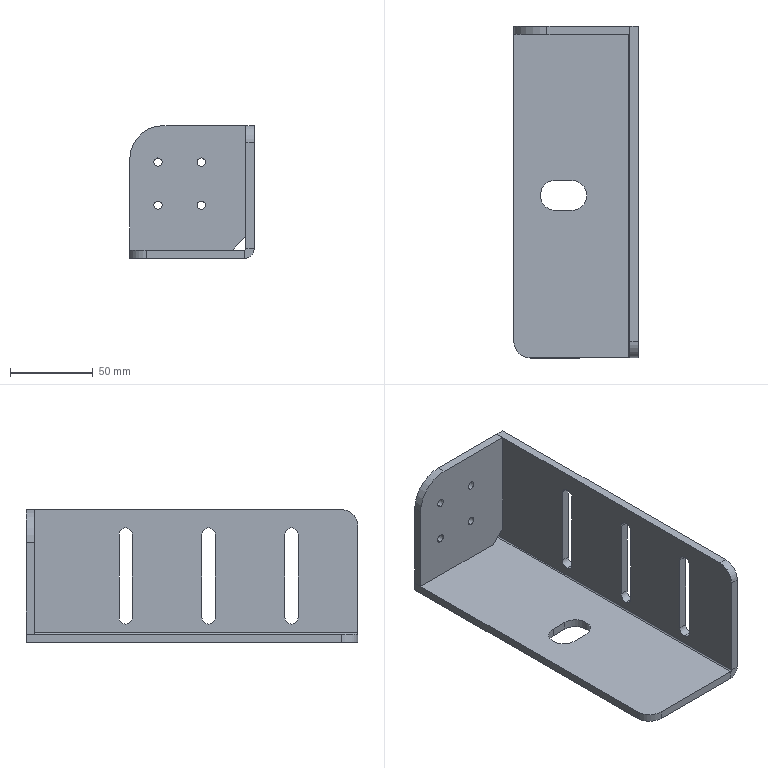Part | SolidWorks | features ICE 4, Fillet 2, EdgeFlange 1, FlatPattern 1, SMBaseFlange 1, SheetMetal 1 | 2 solids | 52 faces | box 75 x 200 x 80 mm | volume 164738 mm3 | plane 27 | cylinder 25 | commonest cylinder face diameters 8 x9 5 x8 18 x3 20 x2 1.473 x1 11.473 x1
STEP:
#1=CARTESIAN_POINT('',(25.,-93.,0.));
#2=VERTEX_POINT('',#1);
#3=CARTESIAN_POINT('',(16.,-102.,0.));
#4=VERTEX_POINT('',#3);
#5=CARTESIAN_POINT('',(25.,-102.,0.));
#6=DIRECTION('',(0.,0.,1.));
#7=DIRECTION('',(1.,0.,0.));
#8=AXIS2_PLACEMENT_3D('',#5,#6,#7);
#9=CIRCLE('',#8,9.);
#10=EDGE_CURVE('',#2,#4,#9,.T.);
#11=ORIENTED_EDGE('',*,*,#10,.T.);
#12=CARTESIAN_POINT('',(16.,-102.,-5.));
#13=VERTEX_POINT('',#12);
#14=CARTESIAN_POINT('',(16.,-102.,75.));
#15=DIRECTION('',(0.,0.,-1.));
#16=VECTOR('',#15,1000.);
#17=LINE('',#14,#16);
#18=EDGE_CURVE('',#4,#13,#17,.T.);
#19=ORIENTED_EDGE('',*,*,#18,.T.);
#20=CARTESIAN_POINT('',(25.,-93.,-5.));
#21=VERTEX_POINT('',#20);
#22=CARTESIAN_POINT('',(25.,-102.,-5.));
#23=DIRECTION('',(0.,0.,-1.));
#24=DIRECTION('',(-1.,0.,0.));
#25=AXIS2_PLACEMENT_3D('',#22,#23,#24);
#26=CIRCLE('',#25,9.);
#27=EDGE_CURVE('',#13,#21,#26,.T.);
#28=ORIENTED_EDGE('',*,*,#27,.T.);
#29=CARTESIAN_POINT('',(25.,-93.,75.));
#30=DIRECTION('',(0.,0.,-1.));
#31=VECTOR('',#30,1000.);
#32=LINE('',#29,#31);
#33=EDGE_CURVE('',#2,#21,#32,.T.);
#34=ORIENTED_EDGE('',*,*,#33,.F.);
#35=EDGE_LOOP('',(#11,#19,#28,#34));
#36=FACE_OUTER_BOUND('',#35,.T.);
#37=CARTESIAN_POINT('',(25.,-102.,75.));
#38=DIRECTION('',(0.,0.,-1.));
#39=DIRECTION('',(-1.,0.,0.));
#40=AXIS2_PLACEMENT_3D('',#37,#38,#39);
#41=CYLINDRICAL_SURFACE('',#40,9.);
#42=ADVANCED_FACE('',(#36),#41,.F.);
#43=CARTESIAN_POINT('',(70.,-56.,10.));
#44=VERTEX_POINT('',#43);
#45=CARTESIAN_POINT('',(70.,-60.,6.));
#46=VERTEX_POINT('',#45);
#47=CARTESIAN_POINT('',(70.,-60.,10.));
#48=DIRECTION('',(-1.,0.,0.));
#49=DIRECTION('',(0.,0.,1.));
#50=AXIS2_PLACEMENT_3D('',#47,#48,#49);
#51=CIRCLE('',#50,4.);
#52=EDGE_CURVE('',#44,#46,#51,.T.);
#53=ORIENTED_EDGE('',*,*,#52,.T.);
#54=CARTESIAN_POINT('',(75.,-60.,6.));
#55=VERTEX_POINT('',#54);
#56=CARTESIAN_POINT('',(65.,-60.,6.));
#57=DIRECTION('',(1.,0.,0.));
#58=VECTOR('',#57,1000.);
#59=LINE('',#56,#58);
#60=EDGE_CURVE('',#46,#55,#59,.T.);
#61=ORIENTED_EDGE('',*,*,#60,.T.);
#62=CARTESIAN_POINT('',(75.,-56.,10.));
#63=VERTEX_POINT('',#62);
#64=CARTESIAN_POINT('',(75.,-60.,10.));
#65=DIRECTION('',(1.,0.,0.));
#66=DIRECTION('',(0.,0.,-1.));
#67=AXIS2_PLACEMENT_3D('',#64,#65,#66);
#68=CIRCLE('',#67,4.);
#69=EDGE_CURVE('',#55,#63,#68,.T.);
#70=ORIENTED_EDGE('',*,*,#69,.T.);
#71=CARTESIAN_POINT('',(65.,-56.,10.));
#72=DIRECTION('',(1.,0.,0.));
#73=VECTOR('',#72,1000.);
#74=LINE('',#71,#73);
#75=EDGE_CURVE('',#44,#63,#74,.T.);
#76=ORIENTED_EDGE('',*,*,#75,.F.);
#77=EDGE_LOOP('',(#53,#61,#70,#76));
#78=FACE_OUTER_BOUND('',#77,.T.);
#79=CARTESIAN_POINT('',(65.,-60.,10.));
#80=DIRECTION('',(1.,0.,0.));
#81=DIRECTION('',(0.,0.,-1.));
#82=AXIS2_PLACEMENT_3D('',#79,#80,#81);
#83=CYLINDRICAL_SURFACE('',#82,4.);
#84=ADVANCED_FACE('',(#78),#83,.F.);
#85=CARTESIAN_POINT('',(70.,-106.,10.));
#86=VERTEX_POINT('',#85);
#87=CARTESIAN_POINT('',(70.,-110.,6.));
#88=VERTEX_POINT('',#87);
#89=CARTESIAN_POINT('',(70.,-110.,10.));
#90=DIRECTION('',(-1.,0.,0.));
#91=DIRECTION('',(0.,0.,1.));
#92=AXIS2_PLACEMENT_3D('',#89,#90,#91);
#93=CIRCLE('',#92,4.);
#94=EDGE_CURVE('',#86,#88,#93,.T.);
#95=ORIENTED_EDGE('',*,*,#94,.T.);
#96=CARTESIAN_POINT('',(75.,-110.,6.));
#97=VERTEX_POINT('',#96);
#98=CARTESIAN_POINT('',(65.,-110.,6.));
#99=DIRECTION('',(1.,0.,0.));
#100=VECTOR('',#99,1000.);
#101=LINE('',#98,#100);
#102=EDGE_CURVE('',#88,#97,#101,.T.);
#103=ORIENTED_EDGE('',*,*,#102,.T.);
#104=CARTESIAN_POINT('',(75.,-106.,10.));
#105=VERTEX_POINT('',#104);
#106=CARTESIAN_POINT('',(75.,-110.,10.));
#107=DIRECTION('',(1.,0.,0.));
#108=DIRECTION('',(0.,0.,-1.));
#109=AXIS2_PLACEMENT_3D('',#106,#107,#108);
#110=CIRCLE('',#109,4.);
#111=EDGE_CURVE('',#97,#105,#110,.T.);
#112=ORIENTED_EDGE('',*,*,#111,.T.);
#113=CARTESIAN_POINT('',(65.,-106.,10.));
#114=DIRECTION('',(1.,0.,0.));
#115=VECTOR('',#114,1000.);
#116=LINE('',#113,#115);
#117=EDGE_CURVE('',#86,#105,#116,.T.);
#118=ORIENTED_EDGE('',*,*,#117,.F.);
#119=EDGE_LOOP('',(#95,#103,#112,#118));
#120=FACE_OUTER_BOUND('',#119,.T.);
#121=CARTESIAN_POINT('',(65.,-110.,10.));
#122=DIRECTION('',(1.,0.,0.));
#123=DIRECTION('',(0.,0.,-1.));
#124=AXIS2_PLACEMENT_3D('',#121,#122,#123);
#125=CYLINDRICAL_SURFACE('',#124,4.);
#126=ADVANCED_FACE('',(#120),#125,.F.);
#127=CARTESIAN_POINT('',(70.,-156.,10.));
#128=VERTEX_POINT('',#127);
#129=CARTESIAN_POINT('',(70.,-160.,6.));
#130=VERTEX_POINT('',#129);
#131=CARTESIAN_POINT('',(70.,-160.,10.));
#132=DIRECTION('',(-1.,0.,0.));
#133=DIRECTION('',(0.,0.,1.));
#134=AXIS2_PLACEMENT_3D('',#131,#132,#133);
#135=CIRCLE('',#134,4.);
#136=EDGE_CURVE('',#128,#130,#135,.T.);
#137=ORIENTED_EDGE('',*,*,#136,.T.);
#138=CARTESIAN_POINT('',(75.,-160.,6.));
#139=VERTEX_POINT('',#138);
#140=CARTESIAN_POINT('',(65.,-160.,6.));
#141=DIRECTION('',(1.,0.,0.));
#142=VECTOR('',#141,1000.);
#143=LINE('',#140,#142);
#144=EDGE_CURVE('',#130,#139,#143,.T.);
#145=ORIENTED_EDGE('',*,*,#144,.T.);
#146=CARTESIAN_POINT('',(75.,-156.,10.));
#147=VERTEX_POINT('',#146);
#148=CARTESIAN_POINT('',(75.,-160.,10.));
#149=DIRECTION('',(1.,0.,0.));
#150=DIRECTION('',(0.,0.,-1.));
#151=AXIS2_PLACEMENT_3D('',#148,#149,#150);
#152=CIRCLE('',#151,4.);
#153=EDGE_CURVE('',#139,#147,#152,.T.);
#154=ORIENTED_EDGE('',*,*,#153,.T.);
#155=CARTESIAN_POINT('',(65.,-156.,10.));
#156=DIRECTION('',(1.,0.,0.));
#157=VECTOR('',#156,1000.);
#158=LINE('',#155,#157);
#159=EDGE_CURVE('',#128,#147,#158,.T.);
#160=ORIENTED_EDGE('',*,*,#159,.F.);
#161=EDGE_LOOP('',(#137,#145,#154,#160));
#162=FACE_OUTER_BOUND('',#161,.T.);
#163=CARTESIAN_POINT('',(65.,-160.,10.));
#164=DIRECTION('',(1.,0.,0.));
#165=DIRECTION('',(0.,0.,-1.));
#166=AXIS2_PLACEMENT_3D('',#163,#164,#165);
#167=CYLINDRICAL_SURFACE('',#166,4.);
#168=ADVANCED_FACE('',(#162),#167,.F.);
#169=CARTESIAN_POINT('',(69.263,0.,0.));
#170=VERTEX_POINT('',#169);
#171=CARTESIAN_POINT('',(0.,0.,0.));
#172=VERTEX_POINT('',#171);
#173=CARTESIAN_POINT('',(0.,0.,0.));
#174=DIRECTION('',(-1.,0.,0.));
#175=VECTOR('',#174,1000.);
#176=LINE('',#173,#175);
#177=EDGE_CURVE('',#170,#172,#176,.T.);
#178=ORIENTED_EDGE('',*,*,#177,.F.);
#179=CARTESIAN_POINT('',(69.263,0.,-5.));
#180=VERTEX_POINT('',#179);
#181=CARTESIAN_POINT('',(69.263,0.,0.));
#182=DIRECTION('',(0.,0.,-1.));
#183=VECTOR('',#182,1000.);
#184=LINE('',#181,#183);
#185=EDGE_CURVE('',#170,#180,#184,.T.);
#186=ORIENTED_EDGE('',*,*,#185,.T.);
#187=CARTESIAN_POINT('',(0.,0.,-5.));
#188=VERTEX_POINT('',#187);
#189=CARTESIAN_POINT('',(0.,0.,-5.));
#190=DIRECTION('',(-1.,0.,0.));
#191=VECTOR('',#190,1000.);
#192=LINE('',#189,#191);
#193=EDGE_CURVE('',#180,#188,#192,.T.);
#194=ORIENTED_EDGE('',*,*,#193,.T.);
#195=CARTESIAN_POINT('',(0.,0.,-5.));
#196=DIRECTION('',(0.,0.,1.));
#197=VECTOR('',#196,1000.);
#198=LINE('',#195,#197);
#199=EDGE_CURVE('',#188,#172,#198,.T.);
#200=ORIENTED_EDGE('',*,*,#199,.T.);
#201=EDGE_LOOP('',(#178,#186,#194,#200));
#202=FACE_OUTER_BOUND('',#201,.T.);
#203=CARTESIAN_POINT('',(0.,0.,-5.));
#204=DIRECTION('',(0.,1.,0.));
#205=DIRECTION('',(0.,0.,1.));
#206=AXIS2_PLACEMENT_3D('',#203,#204,#205);
#207=PLANE('',#206);
#208=ADVANCED_FACE('',(#202),#207,.T.);
#209=CARTESIAN_POINT('',(35.,-111.,-5.));
#210=VERTEX_POINT('',#209);
#211=CARTESIAN_POINT('',(25.,-111.,-5.));
#212=VERTEX_POINT('',#211);
#213=CARTESIAN_POINT('',(35.,-111.,-5.));
#214=DIRECTION('',(-1.,0.,0.));
#215=VECTOR('',#214,1000.);
#216=LINE('',#213,#215);
#217=EDGE_CURVE('',#210,#212,#216,.T.);
#218=ORIENTED_EDGE('',*,*,#217,.F.);
#219=CARTESIAN_POINT('',(35.,-93.,-5.));
#220=VERTEX_POINT('',#219);
#221=CARTESIAN_POINT('',(35.,-102.,-5.));
#222=DIRECTION('',(0.,0.,-1.));
#223=DIRECTION('',(-1.,0.,0.));
#224=AXIS2_PLACEMENT_3D('',#221,#222,#223);
#225=CIRCLE('',#224,9.);
#226=EDGE_CURVE('',#220,#210,#225,.T.);
#227=ORIENTED_EDGE('',*,*,#226,.F.);
#228=CARTESIAN_POINT('',(35.,-93.,-5.));
#229=DIRECTION('',(1.,0.,0.));
#230=VECTOR('',#229,1000.);
#231=LINE('',#228,#230);
#232=EDGE_CURVE('',#21,#220,#231,.T.);
#233=ORIENTED_EDGE('',*,*,#232,.F.);
#234=ORIENTED_EDGE('',*,*,#27,.F.);
#235=CARTESIAN_POINT('',(25.,-102.,-5.));
#236=DIRECTION('',(0.,0.,-1.));
#237=DIRECTION('',(-1.,0.,0.));
#238=AXIS2_PLACEMENT_3D('',#235,#236,#237);
#239=CIRCLE('',#238,9.);
#240=EDGE_CURVE('',#212,#13,#239,.T.);
#241=ORIENTED_EDGE('',*,*,#240,.F.);
#242=EDGE_LOOP('',(#218,#227,#233,#234,#241));
#243=FACE_BOUND('',#242,.T.);
#244=CARTESIAN_POINT('',(10.,-200.,-5.));
#245=VERTEX_POINT('',#244);
#246=CARTESIAN_POINT('',(69.263,-200.,-5.));
#247=VERTEX_POINT('',#246);
#248=CARTESIAN_POINT('',(0.,-200.,-5.));
#249=DIRECTION('',(1.,0.,0.));
#250=VECTOR('',#249,1000.);
#251=LINE('',#248,#250);
#252=EDGE_CURVE('',#245,#247,#251,.T.);
#253=ORIENTED_EDGE('',*,*,#252,.F.);
#254=CARTESIAN_POINT('',(0.,-190.,-5.));
#255=VERTEX_POINT('',#254);
#256=CARTESIAN_POINT('',(10.,-190.,-5.));
#257=DIRECTION('',(0.,0.,-1.));
#258=DIRECTION('',(1.,0.,0.));
#259=AXIS2_PLACEMENT_3D('',#256,#257,#258);
#260=CIRCLE('',#259,10.);
#261=EDGE_CURVE('',#245,#255,#260,.T.);
#262=ORIENTED_EDGE('',*,*,#261,.T.);
#263=CARTESIAN_POINT('',(0.,0.,-5.));
#264=DIRECTION('',(0.,-1.,0.));
#265=VECTOR('',#264,1000.);
#266=LINE('',#263,#265);
#267=EDGE_CURVE('',#188,#255,#266,.T.);
#268=ORIENTED_EDGE('',*,*,#267,.F.);
#269=ORIENTED_EDGE('',*,*,#193,.F.);
#270=CARTESIAN_POINT('',(69.263,0.,-5.));
#271=DIRECTION('',(0.,-1.,0.));
#272=VECTOR('',#271,1000.);
#273=LINE('',#270,#272);
#274=EDGE_CURVE('',#180,#247,#273,.T.);
#275=ORIENTED_EDGE('',*,*,#274,.T.);
#276=EDGE_LOOP('',(#253,#262,#268,#269,#275));
#277=FACE_OUTER_BOUND('',#276,.T.);
#278=CARTESIAN_POINT('',(0.,0.,-5.));
#279=DIRECTION('',(0.,0.,1.));
#280=DIRECTION('',(1.,0.,0.));
#281=AXIS2_PLACEMENT_3D('',#278,#279,#280);
#282=PLANE('',#281);
#283=ADVANCED_FACE('',(#243,#277),#282,.F.);
#284=CARTESIAN_POINT('',(35.,-111.,0.));
#285=VERTEX_POINT('',#284);
#286=CARTESIAN_POINT('',(35.,-93.,0.));
#287=VERTEX_POINT('',#286);
#288=CARTESIAN_POINT('',(35.,-102.,0.));
#289=DIRECTION('',(0.,0.,1.));
#290=DIRECTION('',(1.,0.,0.));
#291=AXIS2_PLACEMENT_3D('',#288,#289,#290);
#292=CIRCLE('',#291,9.);
#293=EDGE_CURVE('',#285,#287,#292,.T.);
#294=ORIENTED_EDGE('',*,*,#293,.F.);
#295=CARTESIAN_POINT('',(25.,-111.,0.));
#296=VERTEX_POINT('',#295);
#297=CARTESIAN_POINT('',(0.,-111.,0.));
#298=DIRECTION('',(1.,0.,0.));
#299=VECTOR('',#298,1000.);
#300=LINE('',#297,#299);
#301=EDGE_CURVE('',#296,#285,#300,.T.);
#302=ORIENTED_EDGE('',*,*,#301,.F.);
#303=CARTESIAN_POINT('',(25.,-102.,0.));
#304=DIRECTION('',(0.,0.,1.));
#305=DIRECTION('',(1.,0.,0.));
#306=AXIS2_PLACEMENT_3D('',#303,#304,#305);
#307=CIRCLE('',#306,9.);
#308=EDGE_CURVE('',#4,#296,#307,.T.);
#309=ORIENTED_EDGE('',*,*,#308,.F.);
#310=ORIENTED_EDGE('',*,*,#10,.F.);
#311=CARTESIAN_POINT('',(0.,-93.,0.));
#312=DIRECTION('',(-1.,0.,0.));
#313=VECTOR('',#312,1000.);
#314=LINE('',#311,#313);
#315=EDGE_CURVE('',#287,#2,#314,.T.);
#316=ORIENTED_EDGE('',*,*,#315,.F.);
#317=EDGE_LOOP('',(#294,#302,#309,#310,#316));
#318=FACE_BOUND('',#317,.T.);
#319=CARTESIAN_POINT('',(0.,-190.,0.));
#320=VERTEX_POINT('',#319);
#321=CARTESIAN_POINT('',(0.,0.,0.));
#322=DIRECTION('',(0.,-1.,0.));
#323=VECTOR('',#322,1000.);
#324=LINE('',#321,#323);
#325=EDGE_CURVE('',#172,#320,#324,.T.);
#326=ORIENTED_EDGE('',*,*,#325,.T.);
#327=CARTESIAN_POINT('',(10.,-200.,0.));
#328=VERTEX_POINT('',#327);
#329=CARTESIAN_POINT('',(10.,-190.,0.));
#330=DIRECTION('',(0.,0.,1.));
#331=DIRECTION('',(1.,0.,0.));
#332=AXIS2_PLACEMENT_3D('',#329,#330,#331);
#333=CIRCLE('',#332,10.);
#334=EDGE_CURVE('',#320,#328,#333,.T.);
#335=ORIENTED_EDGE('',*,*,#334,.T.);
#336=CARTESIAN_POINT('',(69.263,-200.,0.));
#337=VERTEX_POINT('',#336);
#338=CARTESIAN_POINT('',(0.,-200.,0.));
#339=DIRECTION('',(1.,0.,0.));
#340=VECTOR('',#339,1000.);
#341=LINE('',#338,#340);
#342=EDGE_CURVE('',#328,#337,#341,.T.);
#343=ORIENTED_EDGE('',*,*,#342,.T.);
#344=CARTESIAN_POINT('',(69.263,0.,0.));
#345=DIRECTION('',(0.,-1.,0.));
#346=VECTOR('',#345,1000.);
#347=LINE('',#344,#346);
#348=EDGE_CURVE('',#170,#337,#347,.T.);
#349=ORIENTED_EDGE('',*,*,#348,.F.);
#350=ORIENTED_EDGE('',*,*,#177,.T.);
#351=EDGE_LOOP('',(#326,#335,#343,#349,#350));
#352=FACE_OUTER_BOUND('',#351,.T.);
#353=CARTESIAN_POINT('',(0.,0.,0.));
#354=DIRECTION('',(0.,0.,1.));
#355=DIRECTION('',(1.,0.,0.));
#356=AXIS2_PLACEMENT_3D('',#353,#354,#355);
#357=PLANE('',#356);
#358=ADVANCED_FACE('',(#318,#352),#357,.T.);
#359=ORIENTED_EDGE('',*,*,#267,.T.);
#360=CARTESIAN_POINT('',(0.,-190.,-5.));
#361=DIRECTION('',(0.,0.,1.));
#362=VECTOR('',#361,1000.);
#363=LINE('',#360,#362);
#364=EDGE_CURVE('',#255,#320,#363,.T.);
#365=ORIENTED_EDGE('',*,*,#364,.T.);
#366=ORIENTED_EDGE('',*,*,#325,.F.);
#367=ORIENTED_EDGE('',*,*,#199,.F.);
#368=EDGE_LOOP('',(#359,#365,#366,#367));
#369=FACE_OUTER_BOUND('',#368,.T.);
#370=CARTESIAN_POINT('',(0.,0.,-5.));
#371=DIRECTION('',(-1.,0.,0.));
#372=DIRECTION('',(0.,-1.,0.));
#373=AXIS2_PLACEMENT_3D('',#370,#371,#372);
#374=PLANE('',#373);
#375=ADVANCED_FACE('',(#369),#374,.T.);
#376=ORIENTED_EDGE('',*,*,#342,.F.);
#377=CARTESIAN_POINT('',(10.,-200.,-5.));
#378=DIRECTION('',(0.,0.,-1.));
#379=VECTOR('',#378,1000.);
#380=LINE('',#377,#379);
#381=EDGE_CURVE('',#328,#245,#380,.T.);
#382=ORIENTED_EDGE('',*,*,#381,.T.);
#383=ORIENTED_EDGE('',*,*,#252,.T.);
#384=CARTESIAN_POINT('',(69.263,-200.,0.));
#385=DIRECTION('',(0.,0.,-1.));
#386=VECTOR('',#385,1000.);
#387=LINE('',#384,#386);
#388=EDGE_CURVE('',#337,#247,#387,.T.);
#389=ORIENTED_EDGE('',*,*,#388,.F.);
#390=EDGE_LOOP('',(#376,#382,#383,#389));
#391=FACE_OUTER_BOUND('',#390,.T.);
#392=CARTESIAN_POINT('',(0.,-200.,-5.));
#393=DIRECTION('',(0.,-1.,0.));
#394=DIRECTION('',(0.,0.,-1.));
#395=AXIS2_PLACEMENT_3D('',#392,#393,#394);
#396=PLANE('',#395);
#397=ADVANCED_FACE('',(#391),#396,.T.);
#398=CARTESIAN_POINT('',(70.,-200.,0.7366));
#399=VERTEX_POINT('',#398);
#400=CARTESIAN_POINT('',(75.,-200.,0.7366));
#401=VERTEX_POINT('',#400);
#402=CARTESIAN_POINT('',(75.,-200.,0.7366));
#403=DIRECTION('',(1.,0.,0.));
#404=VECTOR('',#403,1000.);
#405=LINE('',#402,#404);
#406=EDGE_CURVE('',#399,#401,#405,.T.);
#407=ORIENTED_EDGE('',*,*,#406,.F.);
#408=CARTESIAN_POINT('',(69.263,-200.,0.7366));
#409=DIRECTION('',(0.,-1.,0.));
#410=DIRECTION('',(0.,0.,1.));
#411=AXIS2_PLACEMENT_3D('',#408,#409,#410);
#412=CIRCLE('',#411,0.7366);
#413=EDGE_CURVE('',#337,#399,#412,.T.);
#414=ORIENTED_EDGE('',*,*,#413,.F.);
#415=ORIENTED_EDGE('',*,*,#388,.T.);
#416=CARTESIAN_POINT('',(69.263,-200.,0.7366));
#417=DIRECTION('',(0.,-1.,0.));
#418=DIRECTION('',(0.,0.,1.));
#419=AXIS2_PLACEMENT_3D('',#416,#417,#418);
#420=CIRCLE('',#419,5.737);
#421=EDGE_CURVE('',#247,#401,#420,.T.);
#422=ORIENTED_EDGE('',*,*,#421,.T.);
#423=EDGE_LOOP('',(#407,#414,#415,#422));
#424=FACE_OUTER_BOUND('',#423,.T.);
#425=CARTESIAN_POINT('',(69.263,-200.,0.7366));
#426=DIRECTION('',(0.,-1.,0.));
#427=DIRECTION('',(0.,0.,-1.));
#428=AXIS2_PLACEMENT_3D('',#425,#426,#427);
#429=PLANE('',#428);
#430=ADVANCED_FACE('',(#424),#429,.T.);
#431=CARTESIAN_POINT('',(70.,0.,0.7366));
#432=VERTEX_POINT('',#431);
#433=CARTESIAN_POINT('',(69.263,0.,0.7366));
#434=DIRECTION('',(0.,1.,0.));
#435=DIRECTION('',(0.,0.,1.));
#436=AXIS2_PLACEMENT_3D('',#433,#434,#435);
#437=CIRCLE('',#436,0.7366);
#438=EDGE_CURVE('',#432,#170,#437,.T.);
#439=ORIENTED_EDGE('',*,*,#438,.F.);
#440=CARTESIAN_POINT('',(75.,0.,0.7366));
#441=VERTEX_POINT('',#440);
#442=CARTESIAN_POINT('',(70.,0.,0.7366));
#443=DIRECTION('',(1.,0.,0.));
#444=VECTOR('',#443,1000.);
#445=LINE('',#442,#444);
#446=EDGE_CURVE('',#432,#441,#445,.T.);
#447=ORIENTED_EDGE('',*,*,#446,.T.);
#448=CARTESIAN_POINT('',(69.263,0.,0.7366));
#449=DIRECTION('',(0.,1.,0.));
#450=DIRECTION('',(0.,0.,1.));
#451=AXIS2_PLACEMENT_3D('',#448,#449,#450);
#452=CIRCLE('',#451,5.737);
#453=EDGE_CURVE('',#441,#180,#452,.T.);
#454=ORIENTED_EDGE('',*,*,#453,.T.);
#455=ORIENTED_EDGE('',*,*,#185,.F.);
#456=EDGE_LOOP('',(#439,#447,#454,#455));
#457=FACE_OUTER_BOUND('',#456,.T.);
#458=CARTESIAN_POINT('',(69.263,0.,0.7366));
#459=DIRECTION('',(0.,-1.,0.));
#460=DIRECTION('',(0.,0.,-1.));
#461=AXIS2_PLACEMENT_3D('',#458,#459,#460);
#462=PLANE('',#461);
#463=ADVANCED_FACE('',(#457),#462,.F.);
#464=ORIENTED_EDGE('',*,*,#274,.F.);
#465=ORIENTED_EDGE('',*,*,#453,.F.);
#466=CARTESIAN_POINT('',(75.,-200.,0.7366));
#467=DIRECTION('',(0.,-1.,0.));
#468=VECTOR('',#467,1000.);
#469=LINE('',#466,#468);
#470=EDGE_CURVE('',#441,#401,#469,.T.);
#471=ORIENTED_EDGE('',*,*,#470,.T.);
#472=ORIENTED_EDGE('',*,*,#421,.F.);
#473=EDGE_LOOP('',(#464,#465,#471,#472));
#474=FACE_OUTER_BOUND('',#473,.T.);
#475=CARTESIAN_POINT('',(69.263,0.,0.7366));
#476=DIRECTION('',(0.,1.,0.));
#477=DIRECTION('',(1.,0.,0.));
#478=AXIS2_PLACEMENT_3D('',#475,#476,#477);
#479=CYLINDRICAL_SURFACE('',#478,5.737);
#480=ADVANCED_FACE('',(#474),#479,.T.);
#481=ORIENTED_EDGE('',*,*,#348,.T.);
#482=ORIENTED_EDGE('',*,*,#413,.T.);
#483=CARTESIAN_POINT('',(70.,-200.,0.7366));
#484=DIRECTION('',(0.,1.,0.));
#485=VECTOR('',#484,1000.);
#486=LINE('',#483,#485);
#487=EDGE_CURVE('',#399,#432,#486,.T.);
#488=ORIENTED_EDGE('',*,*,#487,.T.);
#489=ORIENTED_EDGE('',*,*,#438,.T.);
#490=EDGE_LOOP('',(#481,#482,#488,#489));
#491=FACE_OUTER_BOUND('',#490,.T.);
#492=CARTESIAN_POINT('',(69.263,0.,0.7366));
#493=DIRECTION('',(0.,1.,0.));
#494=DIRECTION('',(1.,0.,0.));
#495=AXIS2_PLACEMENT_3D('',#492,#493,#494);
#496=CYLINDRICAL_SURFACE('',#495,0.7366);
#497=ADVANCED_FACE('',(#491),#496,.F.);
#498=ORIENTED_EDGE('',*,*,#446,.F.);
#499=CARTESIAN_POINT('',(70.,0.,75.));
#500=VERTEX_POINT('',#499);
#501=CARTESIAN_POINT('',(70.,0.,75.));
#502=DIRECTION('',(0.,0.,1.));
#503=VECTOR('',#502,1000.);
#504=LINE('',#501,#503);
#505=EDGE_CURVE('',#432,#500,#504,.T.);
#506=ORIENTED_EDGE('',*,*,#505,.T.);
#507=CARTESIAN_POINT('',(75.,0.,75.));
#508=VERTEX_POINT('',#507);
#509=CARTESIAN_POINT('',(75.,0.,75.));
#510=DIRECTION('',(-1.,0.,0.));
#511=VECTOR('',#510,1000.);
#512=LINE('',#509,#511);
#513=EDGE_CURVE('',#508,#500,#512,.T.);
#514=ORIENTED_EDGE('',*,*,#513,.F.);
#515=CARTESIAN_POINT('',(75.,0.,0.));
#516=DIRECTION('',(0.,0.,1.));
#517=VECTOR('',#516,1000.);
#518=LINE('',#515,#517);
#519=EDGE_CURVE('',#441,#508,#518,.T.);
#520=ORIENTED_EDGE('',*,*,#519,.F.);
#521=EDGE_LOOP('',(#498,#506,#514,#520));
#522=FACE_OUTER_BOUND('',#521,.T.);
#523=CARTESIAN_POINT('',(75.,0.,75.));
#524=DIRECTION('',(0.,-1.,0.));
#525=DIRECTION('',(0.,0.,-1.));
#526=AXIS2_PLACEMENT_3D('',#523,#524,#525);
#527=PLANE('',#526);
#528=ADVANCED_FACE('',(#522),#527,.F.);
#529=CARTESIAN_POINT('',(75.,-200.,65.));
#530=VERTEX_POINT('',#529);
#531=CARTESIAN_POINT('',(75.,-200.,0.));
#532=DIRECTION('',(0.,0.,-1.));
#533=VECTOR('',#532,1000.);
#534=LINE('',#531,#533);
#535=EDGE_CURVE('',#530,#401,#534,.T.);
#536=ORIENTED_EDGE('',*,*,#535,.F.);
#537=CARTESIAN_POINT('',(70.,-200.,65.));
#538=VERTEX_POINT('',#537);
#539=CARTESIAN_POINT('',(75.,-200.,65.));
#540=DIRECTION('',(-1.,0.,0.));
#541=VECTOR('',#540,1000.);
#542=LINE('',#539,#541);
#543=EDGE_CURVE('',#530,#538,#542,.T.);
#544=ORIENTED_EDGE('',*,*,#543,.T.);
#545=CARTESIAN_POINT('',(70.,-200.,0.));
#546=DIRECTION('',(0.,0.,-1.));
#547=VECTOR('',#546,1000.);
#548=LINE('',#545,#547);
#549=EDGE_CURVE('',#538,#399,#548,.T.);
#550=ORIENTED_EDGE('',*,*,#549,.T.);
#551=ORIENTED_EDGE('',*,*,#406,.T.);
#552=EDGE_LOOP('',(#536,#544,#550,#551));
#553=FACE_OUTER_BOUND('',#552,.T.);
#554=CARTESIAN_POINT('',(75.,-200.,0.));
#555=DIRECTION('',(0.,1.,0.));
#556=DIRECTION('',(-1.,0.,0.));
#557=AXIS2_PLACEMENT_3D('',#554,#555,#556);
#558=PLANE('',#557);
#559=ADVANCED_FACE('',(#553),#558,.F.);
#560=CARTESIAN_POINT('',(75.,-64.,60.));
#561=VERTEX_POINT('',#560);
#562=CARTESIAN_POINT('',(75.,-64.,10.));
#563=VERTEX_POINT('',#562);
#564=CARTESIAN_POINT('',(75.,-64.,60.));
#565=DIRECTION('',(0.,0.,-1.));
#566=VECTOR('',#565,1000.);
#567=LINE('',#564,#566);
#568=EDGE_CURVE('',#561,#563,#567,.T.);
#569=ORIENTED_EDGE('',*,*,#568,.F.);
#570=CARTESIAN_POINT('',(75.,-56.,60.));
#571=VERTEX_POINT('',#570);
#572=CARTESIAN_POINT('',(75.,-60.,60.));
#573=DIRECTION('',(1.,0.,0.));
#574=DIRECTION('',(0.,0.,-1.));
#575=AXIS2_PLACEMENT_3D('',#572,#573,#574);
#576=CIRCLE('',#575,4.);
#577=EDGE_CURVE('',#571,#561,#576,.T.);
#578=ORIENTED_EDGE('',*,*,#577,.F.);
#579=CARTESIAN_POINT('',(75.,-56.,60.));
#580=DIRECTION('',(0.,0.,1.));
#581=VECTOR('',#580,1000.);
#582=LINE('',#579,#581);
#583=EDGE_CURVE('',#63,#571,#582,.T.);
#584=ORIENTED_EDGE('',*,*,#583,.F.);
#585=ORIENTED_EDGE('',*,*,#69,.F.);
#586=CARTESIAN_POINT('',(75.,-60.,10.));
#587=DIRECTION('',(1.,0.,0.));
#588=DIRECTION('',(0.,0.,-1.));
#589=AXIS2_PLACEMENT_3D('',#586,#587,#588);
#590=CIRCLE('',#589,4.);
#591=EDGE_CURVE('',#563,#55,#590,.T.);
#592=ORIENTED_EDGE('',*,*,#591,.F.);
#593=EDGE_LOOP('',(#569,#578,#584,#585,#592));
#594=FACE_BOUND('',#593,.T.);
#595=CARTESIAN_POINT('',(75.,-114.,60.));
#596=VERTEX_POINT('',#595);
#597=CARTESIAN_POINT('',(75.,-114.,10.));
#598=VERTEX_POINT('',#597);
#599=CARTESIAN_POINT('',(75.,-114.,60.));
#600=DIRECTION('',(0.,0.,-1.));
#601=VECTOR('',#600,1000.);
#602=LINE('',#599,#601);
#603=EDGE_CURVE('',#596,#598,#602,.T.);
#604=ORIENTED_EDGE('',*,*,#603,.F.);
#605=CARTESIAN_POINT('',(75.,-106.,60.));
#606=VERTEX_POINT('',#605);
#607=CARTESIAN_POINT('',(75.,-110.,60.));
#608=DIRECTION('',(1.,0.,0.));
#609=DIRECTION('',(0.,0.,-1.));
#610=AXIS2_PLACEMENT_3D('',#607,#608,#609);
#611=CIRCLE('',#610,4.);
#612=EDGE_CURVE('',#606,#596,#611,.T.);
#613=ORIENTED_EDGE('',*,*,#612,.F.);
#614=CARTESIAN_POINT('',(75.,-106.,60.));
#615=DIRECTION('',(0.,0.,1.));
#616=VECTOR('',#615,1000.);
#617=LINE('',#614,#616);
#618=EDGE_CURVE('',#105,#606,#617,.T.);
#619=ORIENTED_EDGE('',*,*,#618,.F.);
#620=ORIENTED_EDGE('',*,*,#111,.F.);
#621=CARTESIAN_POINT('',(75.,-110.,10.));
#622=DIRECTION('',(1.,0.,0.));
#623=DIRECTION('',(0.,0.,-1.));
#624=AXIS2_PLACEMENT_3D('',#621,#622,#623);
#625=CIRCLE('',#624,4.);
#626=EDGE_CURVE('',#598,#97,#625,.T.);
#627=ORIENTED_EDGE('',*,*,#626,.F.);
#628=EDGE_LOOP('',(#604,#613,#619,#620,#627));
#629=FACE_BOUND('',#628,.T.);
#630=CARTESIAN_POINT('',(75.,-164.,60.));
#631=VERTEX_POINT('',#630);
#632=CARTESIAN_POINT('',(75.,-164.,10.));
#633=VERTEX_POINT('',#632);
#634=CARTESIAN_POINT('',(75.,-164.,60.));
#635=DIRECTION('',(0.,0.,-1.));
#636=VECTOR('',#635,1000.);
#637=LINE('',#634,#636);
#638=EDGE_CURVE('',#631,#633,#637,.T.);
#639=ORIENTED_EDGE('',*,*,#638,.F.);
#640=CARTESIAN_POINT('',(75.,-156.,60.));
#641=VERTEX_POINT('',#640);
#642=CARTESIAN_POINT('',(75.,-160.,60.));
#643=DIRECTION('',(1.,0.,0.));
#644=DIRECTION('',(0.,0.,-1.));
#645=AXIS2_PLACEMENT_3D('',#642,#643,#644);
#646=CIRCLE('',#645,4.);
#647=EDGE_CURVE('',#641,#631,#646,.T.);
#648=ORIENTED_EDGE('',*,*,#647,.F.);
#649=CARTESIAN_POINT('',(75.,-156.,60.));
#650=DIRECTION('',(0.,0.,1.));
#651=VECTOR('',#650,1000.);
#652=LINE('',#649,#651);
#653=EDGE_CURVE('',#147,#641,#652,.T.);
#654=ORIENTED_EDGE('',*,*,#653,.F.);
#655=ORIENTED_EDGE('',*,*,#153,.F.);
#656=CARTESIAN_POINT('',(75.,-160.,10.));
#657=DIRECTION('',(1.,0.,0.));
#658=DIRECTION('',(0.,0.,-1.));
#659=AXIS2_PLACEMENT_3D('',#656,#657,#658);
#660=CIRCLE('',#659,4.);
#661=EDGE_CURVE('',#633,#139,#660,.T.);
#662=ORIENTED_EDGE('',*,*,#661,.F.);
#663=EDGE_LOOP('',(#639,#648,#654,#655,#662));
#664=FACE_BOUND('',#663,.T.);
#665=CARTESIAN_POINT('',(75.,-190.,75.));
#666=VERTEX_POINT('',#665);
#667=CARTESIAN_POINT('',(75.,0.,75.));
#668=DIRECTION('',(0.,-1.,0.));
#669=VECTOR('',#668,1000.);
#670=LINE('',#667,#669);
#671=EDGE_CURVE('',#508,#666,#670,.T.);
#672=ORIENTED_EDGE('',*,*,#671,.T.);
#673=CARTESIAN_POINT('',(75.,-190.,65.));
#674=DIRECTION('',(1.,0.,0.));
#675=DIRECTION('',(0.,0.,1.));
#676=AXIS2_PLACEMENT_3D('',#673,#674,#675);
#677=CIRCLE('',#676,10.);
#678=EDGE_CURVE('',#666,#530,#677,.T.);
#679=ORIENTED_EDGE('',*,*,#678,.T.);
#680=ORIENTED_EDGE('',*,*,#535,.T.);
#681=ORIENTED_EDGE('',*,*,#470,.F.);
#682=ORIENTED_EDGE('',*,*,#519,.T.);
#683=EDGE_LOOP('',(#672,#679,#680,#681,#682));
#684=FACE_OUTER_BOUND('',#683,.T.);
#685=CARTESIAN_POINT('',(75.,0.,0.));
#686=DIRECTION('',(-1.,0.,0.));
#687=DIRECTION('',(0.,0.,1.));
#688=AXIS2_PLACEMENT_3D('',#685,#686,#687);
#689=PLANE('',#688);
#690=ADVANCED_FACE('',(#594,#629,#664,#684),#689,.F.);
#691=CARTESIAN_POINT('',(70.,-64.,60.));
#692=VERTEX_POINT('',#691);
#693=CARTESIAN_POINT('',(70.,-56.,60.));
#694=VERTEX_POINT('',#693);
#695=CARTESIAN_POINT('',(70.,-60.,60.));
#696=DIRECTION('',(-1.,0.,0.));
#697=DIRECTION('',(0.,0.,1.));
#698=AXIS2_PLACEMENT_3D('',#695,#696,#697);
#699=CIRCLE('',#698,4.);
#700=EDGE_CURVE('',#692,#694,#699,.T.);
#701=ORIENTED_EDGE('',*,*,#700,.F.);
#702=CARTESIAN_POINT('',(70.,-64.,10.));
#703=VERTEX_POINT('',#702);
#704=CARTESIAN_POINT('',(70.,-64.,0.));
#705=DIRECTION('',(0.,0.,1.));
#706=VECTOR('',#705,1000.);
#707=LINE('',#704,#706);
#708=EDGE_CURVE('',#703,#692,#707,.T.);
#709=ORIENTED_EDGE('',*,*,#708,.F.);
#710=CARTESIAN_POINT('',(70.,-60.,10.));
#711=DIRECTION('',(-1.,0.,0.));
#712=DIRECTION('',(0.,0.,1.));
#713=AXIS2_PLACEMENT_3D('',#710,#711,#712);
#714=CIRCLE('',#713,4.);
#715=EDGE_CURVE('',#46,#703,#714,.T.);
#716=ORIENTED_EDGE('',*,*,#715,.F.);
#717=ORIENTED_EDGE('',*,*,#52,.F.);
#718=CARTESIAN_POINT('',(70.,-56.,0.));
#719=DIRECTION('',(0.,0.,-1.));
#720=VECTOR('',#719,1000.);
#721=LINE('',#718,#720);
#722=EDGE_CURVE('',#694,#44,#721,.T.);
#723=ORIENTED_EDGE('',*,*,#722,.F.);
#724=EDGE_LOOP('',(#701,#709,#716,#717,#723));
#725=FACE_BOUND('',#724,.T.);
#726=CARTESIAN_POINT('',(70.,-114.,60.));
#727=VERTEX_POINT('',#726);
#728=CARTESIAN_POINT('',(70.,-106.,60.));
#729=VERTEX_POINT('',#728);
#730=CARTESIAN_POINT('',(70.,-110.,60.));
#731=DIRECTION('',(-1.,0.,0.));
#732=DIRECTION('',(0.,0.,1.));
#733=AXIS2_PLACEMENT_3D('',#730,#731,#732);
#734=CIRCLE('',#733,4.);
#735=EDGE_CURVE('',#727,#729,#734,.T.);
#736=ORIENTED_EDGE('',*,*,#735,.F.);
#737=CARTESIAN_POINT('',(70.,-114.,10.));
#738=VERTEX_POINT('',#737);
#739=CARTESIAN_POINT('',(70.,-114.,0.));
#740=DIRECTION('',(0.,0.,1.));
#741=VECTOR('',#740,1000.);
#742=LINE('',#739,#741);
#743=EDGE_CURVE('',#738,#727,#742,.T.);
#744=ORIENTED_EDGE('',*,*,#743,.F.);
#745=CARTESIAN_POINT('',(70.,-110.,10.));
#746=DIRECTION('',(-1.,0.,0.));
#747=DIRECTION('',(0.,0.,1.));
#748=AXIS2_PLACEMENT_3D('',#745,#746,#747);
#749=CIRCLE('',#748,4.);
#750=EDGE_CURVE('',#88,#738,#749,.T.);
#751=ORIENTED_EDGE('',*,*,#750,.F.);
#752=ORIENTED_EDGE('',*,*,#94,.F.);
#753=CARTESIAN_POINT('',(70.,-106.,0.));
#754=DIRECTION('',(0.,0.,-1.));
#755=VECTOR('',#754,1000.);
#756=LINE('',#753,#755);
#757=EDGE_CURVE('',#729,#86,#756,.T.);
#758=ORIENTED_EDGE('',*,*,#757,.F.);
#759=EDGE_LOOP('',(#736,#744,#751,#752,#758));
#760=FACE_BOUND('',#759,.T.);
#761=CARTESIAN_POINT('',(70.,-164.,60.));
#762=VERTEX_POINT('',#761);
#763=CARTESIAN_POINT('',(70.,-156.,60.));
#764=VERTEX_POINT('',#763);
#765=CARTESIAN_POINT('',(70.,-160.,60.));
#766=DIRECTION('',(-1.,0.,0.));
#767=DIRECTION('',(0.,0.,1.));
#768=AXIS2_PLACEMENT_3D('',#765,#766,#767);
#769=CIRCLE('',#768,4.);
#770=EDGE_CURVE('',#762,#764,#769,.T.);
#771=ORIENTED_EDGE('',*,*,#770,.F.);
#772=CARTESIAN_POINT('',(70.,-164.,10.));
#773=VERTEX_POINT('',#772);
#774=CARTESIAN_POINT('',(70.,-164.,0.));
#775=DIRECTION('',(0.,0.,1.));
#776=VECTOR('',#775,1000.);
#777=LINE('',#774,#776);
#778=EDGE_CURVE('',#773,#762,#777,.T.);
#779=ORIENTED_EDGE('',*,*,#778,.F.);
#780=CARTESIAN_POINT('',(70.,-160.,10.));
#781=DIRECTION('',(-1.,0.,0.));
#782=DIRECTION('',(0.,0.,1.));
#783=AXIS2_PLACEMENT_3D('',#780,#781,#782);
#784=CIRCLE('',#783,4.);
#785=EDGE_CURVE('',#130,#773,#784,.T.);
#786=ORIENTED_EDGE('',*,*,#785,.F.);
#787=ORIENTED_EDGE('',*,*,#136,.F.);
#788=CARTESIAN_POINT('',(70.,-156.,0.));
#789=DIRECTION('',(0.,0.,-1.));
#790=VECTOR('',#789,1000.);
#791=LINE('',#788,#790);
#792=EDGE_CURVE('',#764,#128,#791,.T.);
#793=ORIENTED_EDGE('',*,*,#792,.F.);
#794=EDGE_LOOP('',(#771,#779,#786,#787,#793));
#795=FACE_BOUND('',#794,.T.);
#796=ORIENTED_EDGE('',*,*,#549,.F.);
#797=CARTESIAN_POINT('',(70.,-190.,75.));
#798=VERTEX_POINT('',#797);
#799=CARTESIAN_POINT('',(70.,-190.,65.));
#800=DIRECTION('',(-1.,0.,0.));
#801=DIRECTION('',(0.,0.,1.));
#802=AXIS2_PLACEMENT_3D('',#799,#800,#801);
#803=CIRCLE('',#802,10.);
#804=EDGE_CURVE('',#538,#798,#803,.T.);
#805=ORIENTED_EDGE('',*,*,#804,.T.);
#806=CARTESIAN_POINT('',(70.,-200.,75.));
#807=DIRECTION('',(0.,-1.,0.));
#808=VECTOR('',#807,1000.);
#809=LINE('',#806,#808);
#810=EDGE_CURVE('',#500,#798,#809,.T.);
#811=ORIENTED_EDGE('',*,*,#810,.F.);
#812=ORIENTED_EDGE('',*,*,#505,.F.);
#813=ORIENTED_EDGE('',*,*,#487,.F.);
#814=EDGE_LOOP('',(#796,#805,#811,#812,#813));
#815=FACE_OUTER_BOUND('',#814,.T.);
#816=CARTESIAN_POINT('',(70.,0.,0.));
#817=DIRECTION('',(-1.,0.,0.));
#818=DIRECTION('',(0.,0.,1.));
#819=AXIS2_PLACEMENT_3D('',#816,#817,#818);
#820=PLANE('',#819);
#821=ADVANCED_FACE('',(#725,#760,#795,#815),#820,.T.);
#822=ORIENTED_EDGE('',*,*,#810,.T.);
#823=CARTESIAN_POINT('',(75.,-190.,75.));
#824=DIRECTION('',(1.,0.,0.));
#825=VECTOR('',#824,1000.);
#826=LINE('',#823,#825);
#827=EDGE_CURVE('',#798,#666,#826,.T.);
#828=ORIENTED_EDGE('',*,*,#827,.T.);
#829=ORIENTED_EDGE('',*,*,#671,.F.);
#830=ORIENTED_EDGE('',*,*,#513,.T.);
#831=EDGE_LOOP('',(#822,#828,#829,#830));
#832=FACE_OUTER_BOUND('',#831,.T.);
#833=CARTESIAN_POINT('',(75.,-200.,75.));
#834=DIRECTION('',(0.,0.,-1.));
#835=DIRECTION('',(-1.,0.,0.));
#836=AXIS2_PLACEMENT_3D('',#833,#834,#835);
#837=PLANE('',#836);
#838=ADVANCED_FACE('',(#832),#837,.F.);
#839=ORIENTED_EDGE('',*,*,#770,.T.);
#840=CARTESIAN_POINT('',(65.,-156.,60.));
#841=DIRECTION('',(1.,0.,0.));
#842=VECTOR('',#841,1000.);
#843=LINE('',#840,#842);
#844=EDGE_CURVE('',#764,#641,#843,.T.);
#845=ORIENTED_EDGE('',*,*,#844,.T.);
#846=ORIENTED_EDGE('',*,*,#647,.T.);
#847=CARTESIAN_POINT('',(65.,-164.,60.));
#848=DIRECTION('',(1.,0.,0.));
#849=VECTOR('',#848,1000.);
#850=LINE('',#847,#849);
#851=EDGE_CURVE('',#762,#631,#850,.T.);
#852=ORIENTED_EDGE('',*,*,#851,.F.);
#853=EDGE_LOOP('',(#839,#845,#846,#852));
#854=FACE_OUTER_BOUND('',#853,.T.);
#855=CARTESIAN_POINT('',(65.,-160.,60.));
#856=DIRECTION('',(1.,0.,0.));
#857=DIRECTION('',(0.,0.,-1.));
#858=AXIS2_PLACEMENT_3D('',#855,#856,#857);
#859=CYLINDRICAL_SURFACE('',#858,4.);
#860=ADVANCED_FACE('',(#854),#859,.F.);
#861=ORIENTED_EDGE('',*,*,#792,.T.);
#862=ORIENTED_EDGE('',*,*,#159,.T.);
#863=ORIENTED_EDGE('',*,*,#653,.T.);
#864=ORIENTED_EDGE('',*,*,#844,.F.);
#865=EDGE_LOOP('',(#861,#862,#863,#864));
#866=FACE_OUTER_BOUND('',#865,.T.);
#867=CARTESIAN_POINT('',(65.,-156.,60.));
#868=DIRECTION('',(0.,1.,0.));
#869=DIRECTION('',(-1.,0.,0.));
#870=AXIS2_PLACEMENT_3D('',#867,#868,#869);
#871=PLANE('',#870);
#872=ADVANCED_FACE('',(#866),#871,.F.);
#873=ORIENTED_EDGE('',*,*,#144,.F.);
#874=ORIENTED_EDGE('',*,*,#785,.T.);
#875=CARTESIAN_POINT('',(65.,-164.,10.));
#876=DIRECTION('',(1.,0.,0.));
#877=VECTOR('',#876,1000.);
#878=LINE('',#875,#877);
#879=EDGE_CURVE('',#773,#633,#878,.T.);
#880=ORIENTED_EDGE('',*,*,#879,.T.);
#881=ORIENTED_EDGE('',*,*,#661,.T.);
#882=EDGE_LOOP('',(#873,#874,#880,#881));
#883=FACE_OUTER_BOUND('',#882,.T.);
#884=CARTESIAN_POINT('',(65.,-160.,10.));
#885=DIRECTION('',(1.,0.,0.));
#886=DIRECTION('',(0.,0.,-1.));
#887=AXIS2_PLACEMENT_3D('',#884,#885,#886);
#888=CYLINDRICAL_SURFACE('',#887,4.);
#889=ADVANCED_FACE('',(#883),#888,.F.);
#890=ORIENTED_EDGE('',*,*,#778,.T.);
#891=ORIENTED_EDGE('',*,*,#851,.T.);
#892=ORIENTED_EDGE('',*,*,#638,.T.);
#893=ORIENTED_EDGE('',*,*,#879,.F.);
#894=EDGE_LOOP('',(#890,#891,#892,#893));
#895=FACE_OUTER_BOUND('',#894,.T.);
#896=CARTESIAN_POINT('',(65.,-164.,60.));
#897=DIRECTION('',(0.,-1.,0.));
#898=DIRECTION('',(1.,0.,0.));
#899=AXIS2_PLACEMENT_3D('',#896,#897,#898);
#900=PLANE('',#899);
#901=ADVANCED_FACE('',(#895),#900,.F.);
#902=ORIENTED_EDGE('',*,*,#735,.T.);
#903=CARTESIAN_POINT('',(65.,-106.,60.));
#904=DIRECTION('',(1.,0.,0.));
#905=VECTOR('',#904,1000.);
#906=LINE('',#903,#905);
#907=EDGE_CURVE('',#729,#606,#906,.T.);
#908=ORIENTED_EDGE('',*,*,#907,.T.);
#909=ORIENTED_EDGE('',*,*,#612,.T.);
#910=CARTESIAN_POINT('',(65.,-114.,60.));
#911=DIRECTION('',(1.,0.,0.));
#912=VECTOR('',#911,1000.);
#913=LINE('',#910,#912);
#914=EDGE_CURVE('',#727,#596,#913,.T.);
#915=ORIENTED_EDGE('',*,*,#914,.F.);
#916=EDGE_LOOP('',(#902,#908,#909,#915));
#917=FACE_OUTER_BOUND('',#916,.T.);
#918=CARTESIAN_POINT('',(65.,-110.,60.));
#919=DIRECTION('',(1.,0.,0.));
#920=DIRECTION('',(0.,0.,-1.));
#921=AXIS2_PLACEMENT_3D('',#918,#919,#920);
#922=CYLINDRICAL_SURFACE('',#921,4.);
#923=ADVANCED_FACE('',(#917),#922,.F.);
#924=ORIENTED_EDGE('',*,*,#757,.T.);
#925=ORIENTED_EDGE('',*,*,#117,.T.);
#926=ORIENTED_EDGE('',*,*,#618,.T.);
#927=ORIENTED_EDGE('',*,*,#907,.F.);
#928=EDGE_LOOP('',(#924,#925,#926,#927));
#929=FACE_OUTER_BOUND('',#928,.T.);
#930=CARTESIAN_POINT('',(65.,-106.,60.));
#931=DIRECTION('',(0.,1.,0.));
#932=DIRECTION('',(-1.,0.,0.));
#933=AXIS2_PLACEMENT_3D('',#930,#931,#932);
#934=PLANE('',#933);
#935=ADVANCED_FACE('',(#929),#934,.F.);
#936=ORIENTED_EDGE('',*,*,#102,.F.);
#937=ORIENTED_EDGE('',*,*,#750,.T.);
#938=CARTESIAN_POINT('',(65.,-114.,10.));
#939=DIRECTION('',(1.,0.,0.));
#940=VECTOR('',#939,1000.);
#941=LINE('',#938,#940);
#942=EDGE_CURVE('',#738,#598,#941,.T.);
#943=ORIENTED_EDGE('',*,*,#942,.T.);
#944=ORIENTED_EDGE('',*,*,#626,.T.);
#945=EDGE_LOOP('',(#936,#937,#943,#944));
#946=FACE_OUTER_BOUND('',#945,.T.);
#947=CARTESIAN_POINT('',(65.,-110.,10.));
#948=DIRECTION('',(1.,0.,0.));
#949=DIRECTION('',(0.,0.,-1.));
#950=AXIS2_PLACEMENT_3D('',#947,#948,#949);
#951=CYLINDRICAL_SURFACE('',#950,4.);
#952=ADVANCED_FACE('',(#946),#951,.F.);
#953=ORIENTED_EDGE('',*,*,#743,.T.);
#954=ORIENTED_EDGE('',*,*,#914,.T.);
#955=ORIENTED_EDGE('',*,*,#603,.T.);
#956=ORIENTED_EDGE('',*,*,#942,.F.);
#957=EDGE_LOOP('',(#953,#954,#955,#956));
#958=FACE_OUTER_BOUND('',#957,.T.);
#959=CARTESIAN_POINT('',(65.,-114.,60.));
#960=DIRECTION('',(0.,-1.,0.));
#961=DIRECTION('',(1.,0.,0.));
#962=AXIS2_PLACEMENT_3D('',#959,#960,#961);
#963=PLANE('',#962);
#964=ADVANCED_FACE('',(#958),#963,.F.);
#965=ORIENTED_EDGE('',*,*,#700,.T.);
#966=CARTESIAN_POINT('',(65.,-56.,60.));
#967=DIRECTION('',(1.,0.,0.));
#968=VECTOR('',#967,1000.);
#969=LINE('',#966,#968);
#970=EDGE_CURVE('',#694,#571,#969,.T.);
#971=ORIENTED_EDGE('',*,*,#970,.T.);
#972=ORIENTED_EDGE('',*,*,#577,.T.);
#973=CARTESIAN_POINT('',(65.,-64.,60.));
#974=DIRECTION('',(1.,0.,0.));
#975=VECTOR('',#974,1000.);
#976=LINE('',#973,#975);
#977=EDGE_CURVE('',#692,#561,#976,.T.);
#978=ORIENTED_EDGE('',*,*,#977,.F.);
#979=EDGE_LOOP('',(#965,#971,#972,#978));
#980=FACE_OUTER_BOUND('',#979,.T.);
#981=CARTESIAN_POINT('',(65.,-60.,60.));
#982=DIRECTION('',(1.,0.,0.));
#983=DIRECTION('',(0.,0.,-1.));
#984=AXIS2_PLACEMENT_3D('',#981,#982,#983);
#985=CYLINDRICAL_SURFACE('',#984,4.);
#986=ADVANCED_FACE('',(#980),#985,.F.);
#987=ORIENTED_EDGE('',*,*,#722,.T.);
#988=ORIENTED_EDGE('',*,*,#75,.T.);
#989=ORIENTED_EDGE('',*,*,#583,.T.);
#990=ORIENTED_EDGE('',*,*,#970,.F.);
#991=EDGE_LOOP('',(#987,#988,#989,#990));
#992=FACE_OUTER_BOUND('',#991,.T.);
#993=CARTESIAN_POINT('',(65.,-56.,60.));
#994=DIRECTION('',(0.,1.,0.));
#995=DIRECTION('',(-1.,0.,0.));
#996=AXIS2_PLACEMENT_3D('',#993,#994,#995);
#997=PLANE('',#996);
#998=ADVANCED_FACE('',(#992),#997,.F.);
#999=ORIENTED_EDGE('',*,*,#60,.F.);
#1000=ORIENTED_EDGE('',*,*,#715,.T.);
#1001=CARTESIAN_POINT('',(65.,-64.,10.));
#1002=DIRECTION('',(1.,0.,0.));
#1003=VECTOR('',#1002,1000.);
#1004=LINE('',#1001,#1003);
#1005=EDGE_CURVE('',#703,#563,#1004,.T.);
#1006=ORIENTED_EDGE('',*,*,#1005,.T.);
#1007=ORIENTED_EDGE('',*,*,#591,.T.);
#1008=EDGE_LOOP('',(#999,#1000,#1006,#1007));
#1009=FACE_OUTER_BOUND('',#1008,.T.);
#1010=CARTESIAN_POINT('',(65.,-60.,10.));
#1011=DIRECTION('',(1.,0.,0.));
#1012=DIRECTION('',(0.,0.,-1.));
#1013=AXIS2_PLACEMENT_3D('',#1010,#1011,#1012);
#1014=CYLINDRICAL_SURFACE('',#1013,4.);
#1015=ADVANCED_FACE('',(#1009),#1014,.F.);
#1016=ORIENTED_EDGE('',*,*,#708,.T.);
#1017=ORIENTED_EDGE('',*,*,#977,.T.);
#1018=ORIENTED_EDGE('',*,*,#568,.T.);
#1019=ORIENTED_EDGE('',*,*,#1005,.F.);
#1020=EDGE_LOOP('',(#1016,#1017,#1018,#1019));
#1021=FACE_OUTER_BOUND('',#1020,.T.);
#1022=CARTESIAN_POINT('',(65.,-64.,60.));
#1023=DIRECTION('',(0.,-1.,0.));
#1024=DIRECTION('',(1.,0.,0.));
#1025=AXIS2_PLACEMENT_3D('',#1022,#1023,#1024);
#1026=PLANE('',#1025);
#1027=ADVANCED_FACE('',(#1021),#1026,.F.);
#1028=ORIENTED_EDGE('',*,*,#293,.T.);
#1029=CARTESIAN_POINT('',(35.,-93.,75.));
#1030=DIRECTION('',(0.,0.,-1.));
#1031=VECTOR('',#1030,1000.);
#1032=LINE('',#1029,#1031);
#1033=EDGE_CURVE('',#287,#220,#1032,.T.);
#1034=ORIENTED_EDGE('',*,*,#1033,.T.);
#1035=ORIENTED_EDGE('',*,*,#226,.T.);
#1036=CARTESIAN_POINT('',(35.,-111.,75.));
#1037=DIRECTION('',(0.,0.,-1.));
#1038=VECTOR('',#1037,1000.);
#1039=LINE('',#1036,#1038);
#1040=EDGE_CURVE('',#285,#210,#1039,.T.);
#1041=ORIENTED_EDGE('',*,*,#1040,.F.);
#1042=EDGE_LOOP('',(#1028,#1034,#1035,#1041));
#1043=FACE_OUTER_BOUND('',#1042,.T.);
#1044=CARTESIAN_POINT('',(35.,-102.,75.));
#1045=DIRECTION('',(0.,0.,-1.));
#1046=DIRECTION('',(-1.,0.,0.));
#1047=AXIS2_PLACEMENT_3D('',#1044,#1045,#1046);
#1048=CYLINDRICAL_SURFACE('',#1047,9.);
#1049=ADVANCED_FACE('',(#1043),#1048,.F.);
#1050=ORIENTED_EDGE('',*,*,#315,.T.);
#1051=ORIENTED_EDGE('',*,*,#33,.T.);
#1052=ORIENTED_EDGE('',*,*,#232,.T.);
#1053=ORIENTED_EDGE('',*,*,#1033,.F.);
#1054=EDGE_LOOP('',(#1050,#1051,#1052,#1053));
#1055=FACE_OUTER_BOUND('',#1054,.T.);
#1056=CARTESIAN_POINT('',(35.,-93.,75.));
#1057=DIRECTION('',(0.,1.,0.));
#1058=DIRECTION('',(0.,0.,1.));
#1059=AXIS2_PLACEMENT_3D('',#1056,#1057,#1058);
#1060=PLANE('',#1059);
#1061=ADVANCED_FACE('',(#1055),#1060,.F.);
#1062=ORIENTED_EDGE('',*,*,#18,.F.);
#1063=ORIENTED_EDGE('',*,*,#308,.T.);
#1064=CARTESIAN_POINT('',(25.,-111.,75.));
#1065=DIRECTION('',(0.,0.,-1.));
#1066=VECTOR('',#1065,1000.);
#1067=LINE('',#1064,#1066);
#1068=EDGE_CURVE('',#296,#212,#1067,.T.);
#1069=ORIENTED_EDGE('',*,*,#1068,.T.);
#1070=ORIENTED_EDGE('',*,*,#240,.T.);
#1071=EDGE_LOOP('',(#1062,#1063,#1069,#1070));
#1072=FACE_OUTER_BOUND('',#1071,.T.);
#1073=CARTESIAN_POINT('',(25.,-102.,75.));
#1074=DIRECTION('',(0.,0.,-1.));
#1075=DIRECTION('',(-1.,0.,0.));
#1076=AXIS2_PLACEMENT_3D('',#1073,#1074,#1075);
#1077=CYLINDRICAL_SURFACE('',#1076,9.);
#1078=ADVANCED_FACE('',(#1072),#1077,.F.);
#1079=ORIENTED_EDGE('',*,*,#301,.T.);
#1080=ORIENTED_EDGE('',*,*,#1040,.T.);
#1081=ORIENTED_EDGE('',*,*,#217,.T.);
#1082=ORIENTED_EDGE('',*,*,#1068,.F.);
#1083=EDGE_LOOP('',(#1079,#1080,#1081,#1082));
#1084=FACE_OUTER_BOUND('',#1083,.T.);
#1085=CARTESIAN_POINT('',(35.,-111.,75.));
#1086=DIRECTION('',(0.,-1.,0.));
#1087=DIRECTION('',(0.,0.,-1.));
#1088=AXIS2_PLACEMENT_3D('',#1085,#1086,#1087);
#1089=PLANE('',#1088);
#1090=ADVANCED_FACE('',(#1084),#1089,.F.);
#1091=ORIENTED_EDGE('',*,*,#261,.F.);
#1092=ORIENTED_EDGE('',*,*,#381,.F.);
#1093=ORIENTED_EDGE('',*,*,#334,.F.);
#1094=ORIENTED_EDGE('',*,*,#364,.F.);
#1095=EDGE_LOOP('',(#1091,#1092,#1093,#1094));
#1096=FACE_OUTER_BOUND('',#1095,.T.);
#1097=CARTESIAN_POINT('',(10.,-190.,-5.));
#1098=DIRECTION('',(0.,0.,1.));
#1099=DIRECTION('',(1.,0.,0.));
#1100=AXIS2_PLACEMENT_3D('',#1097,#1098,#1099);
#1101=CYLINDRICAL_SURFACE('',#1100,10.);
#1102=ADVANCED_FACE('',(#1096),#1101,.T.);
#1103=ORIENTED_EDGE('',*,*,#678,.F.);
#1104=ORIENTED_EDGE('',*,*,#827,.F.);
#1105=ORIENTED_EDGE('',*,*,#804,.F.);
#1106=ORIENTED_EDGE('',*,*,#543,.F.);
#1107=EDGE_LOOP('',(#1103,#1104,#1105,#1106));
#1108=FACE_OUTER_BOUND('',#1107,.T.);
#1109=CARTESIAN_POINT('',(75.,-190.,65.));
#1110=DIRECTION('',(-1.,0.,0.));
#1111=DIRECTION('',(0.,0.,1.));
#1112=AXIS2_PLACEMENT_3D('',#1109,#1110,#1111);
#1113=CYLINDRICAL_SURFACE('',#1112,10.);
#1114=ADVANCED_FACE('',(#1108),#1113,.T.);
#1115=CLOSED_SHELL('',(#42,#84,#126,#168,#208,#283,#358,#375,#397,#430,#463,#480,#497,#528,#559,#690,#821,#838,#860,#872,#889,#901,#923,#935,#952,#964,#986,#998,#1015,#1027,#1049,#1061,#1078,#1090,#1102,#1114));
#1116=MANIFOLD_SOLID_BREP('',#1115);
#1117=CARTESIAN_POINT('',(17.,-5.,24.5));
#1118=VERTEX_POINT('',#1117);
#1119=CARTESIAN_POINT('',(17.,-5.,29.5));
#1120=VERTEX_POINT('',#1119);
#1121=CARTESIAN_POINT('',(17.,-5.,27.));
#1122=DIRECTION('',(0.,1.,0.));
#1123=DIRECTION('',(0.,0.,1.));
#1124=AXIS2_PLACEMENT_3D('',#1121,#1122,#1123);
#1125=CIRCLE('',#1124,2.5);
#1126=EDGE_CURVE('',#1118,#1120,#1125,.T.);
#1127=ORIENTED_EDGE('',*,*,#1126,.F.);
#1128=CARTESIAN_POINT('',(17.,0.,24.5));
#1129=VERTEX_POINT('',#1128);
#1130=CARTESIAN_POINT('',(17.,-200.,24.5));
#1131=DIRECTION('',(0.,1.,0.));
#1132=VECTOR('',#1131,1000.);
#1133=LINE('',#1130,#1132);
#1134=EDGE_CURVE('',#1118,#1129,#1133,.T.);
#1135=ORIENTED_EDGE('',*,*,#1134,.T.);
#1136=CARTESIAN_POINT('',(17.,0.,29.5));
#1137=VERTEX_POINT('',#1136);
#1138=CARTESIAN_POINT('',(17.,0.,27.));
#1139=DIRECTION('',(0.,1.,0.));
#1140=DIRECTION('',(0.,0.,1.));
#1141=AXIS2_PLACEMENT_3D('',#1138,#1139,#1140);
#1142=CIRCLE('',#1141,2.5);
#1143=EDGE_CURVE('',#1129,#1137,#1142,.T.);
#1144=ORIENTED_EDGE('',*,*,#1143,.T.);
#1145=CARTESIAN_POINT('',(17.,-200.,29.5));
#1146=DIRECTION('',(0.,1.,0.));
#1147=VECTOR('',#1146,1000.);
#1148=LINE('',#1145,#1147);
#1149=EDGE_CURVE('',#1120,#1137,#1148,.T.);
#1150=ORIENTED_EDGE('',*,*,#1149,.F.);
#1151=EDGE_LOOP('',(#1127,#1135,#1144,#1150));
#1152=FACE_OUTER_BOUND('',#1151,.T.);
#1153=CARTESIAN_POINT('',(17.,-200.,27.));
#1154=DIRECTION('',(0.,1.,0.));
#1155=DIRECTION('',(0.,0.,1.));
#1156=AXIS2_PLACEMENT_3D('',#1153,#1154,#1155);
#1157=CYLINDRICAL_SURFACE('',#1156,2.5);
#1158=ADVANCED_FACE('',(#1152),#1157,.F.);
#1159=CARTESIAN_POINT('',(43.,-5.,50.5));
#1160=VERTEX_POINT('',#1159);
#1161=CARTESIAN_POINT('',(43.,-5.,55.5));
#1162=VERTEX_POINT('',#1161);
#1163=CARTESIAN_POINT('',(43.,-5.,53.));
#1164=DIRECTION('',(0.,1.,0.));
#1165=DIRECTION('',(0.,0.,1.));
#1166=AXIS2_PLACEMENT_3D('',#1163,#1164,#1165);
#1167=CIRCLE('',#1166,2.5);
#1168=EDGE_CURVE('',#1160,#1162,#1167,.T.);
#1169=ORIENTED_EDGE('',*,*,#1168,.F.);
#1170=CARTESIAN_POINT('',(43.,0.,50.5));
#1171=VERTEX_POINT('',#1170);
#1172=CARTESIAN_POINT('',(43.,-200.,50.5));
#1173=DIRECTION('',(0.,1.,0.));
#1174=VECTOR('',#1173,1000.);
#1175=LINE('',#1172,#1174);
#1176=EDGE_CURVE('',#1160,#1171,#1175,.T.);
#1177=ORIENTED_EDGE('',*,*,#1176,.T.);
#1178=CARTESIAN_POINT('',(43.,0.,55.5));
#1179=VERTEX_POINT('',#1178);
#1180=CARTESIAN_POINT('',(43.,0.,53.));
#1181=DIRECTION('',(0.,1.,0.));
#1182=DIRECTION('',(0.,0.,1.));
#1183=AXIS2_PLACEMENT_3D('',#1180,#1181,#1182);
#1184=CIRCLE('',#1183,2.5);
#1185=EDGE_CURVE('',#1171,#1179,#1184,.T.);
#1186=ORIENTED_EDGE('',*,*,#1185,.T.);
#1187=CARTESIAN_POINT('',(43.,-200.,55.5));
#1188=DIRECTION('',(0.,1.,0.));
#1189=VECTOR('',#1188,1000.);
#1190=LINE('',#1187,#1189);
#1191=EDGE_CURVE('',#1162,#1179,#1190,.T.);
#1192=ORIENTED_EDGE('',*,*,#1191,.F.);
#1193=EDGE_LOOP('',(#1169,#1177,#1186,#1192));
#1194=FACE_OUTER_BOUND('',#1193,.T.);
#1195=CARTESIAN_POINT('',(43.,-200.,53.));
#1196=DIRECTION('',(0.,1.,0.));
#1197=DIRECTION('',(0.,0.,1.));
#1198=AXIS2_PLACEMENT_3D('',#1195,#1196,#1197);
#1199=CYLINDRICAL_SURFACE('',#1198,2.5);
#1200=ADVANCED_FACE('',(#1194),#1199,.F.);
#1201=CARTESIAN_POINT('',(17.,-5.,50.5));
#1202=VERTEX_POINT('',#1201);
#1203=CARTESIAN_POINT('',(17.,-5.,55.5));
#1204=VERTEX_POINT('',#1203);
#1205=CARTESIAN_POINT('',(17.,-5.,53.));
#1206=DIRECTION('',(0.,1.,0.));
#1207=DIRECTION('',(0.,0.,1.));
#1208=AXIS2_PLACEMENT_3D('',#1205,#1206,#1207);
#1209=CIRCLE('',#1208,2.5);
#1210=EDGE_CURVE('',#1202,#1204,#1209,.T.);
#1211=ORIENTED_EDGE('',*,*,#1210,.F.);
#1212=CARTESIAN_POINT('',(17.,0.,50.5));
#1213=VERTEX_POINT('',#1212);
#1214=CARTESIAN_POINT('',(17.,-200.,50.5));
#1215=DIRECTION('',(0.,1.,0.));
#1216=VECTOR('',#1215,1000.);
#1217=LINE('',#1214,#1216);
#1218=EDGE_CURVE('',#1202,#1213,#1217,.T.);
#1219=ORIENTED_EDGE('',*,*,#1218,.T.);
#1220=CARTESIAN_POINT('',(17.,0.,55.5));
#1221=VERTEX_POINT('',#1220);
#1222=CARTESIAN_POINT('',(17.,0.,53.));
#1223=DIRECTION('',(0.,1.,0.));
#1224=DIRECTION('',(0.,0.,1.));
#1225=AXIS2_PLACEMENT_3D('',#1222,#1223,#1224);
#1226=CIRCLE('',#1225,2.5);
#1227=EDGE_CURVE('',#1213,#1221,#1226,.T.);
#1228=ORIENTED_EDGE('',*,*,#1227,.T.);
#1229=CARTESIAN_POINT('',(17.,-200.,55.5));
#1230=DIRECTION('',(0.,1.,0.));
#1231=VECTOR('',#1230,1000.);
#1232=LINE('',#1229,#1231);
#1233=EDGE_CURVE('',#1204,#1221,#1232,.T.);
#1234=ORIENTED_EDGE('',*,*,#1233,.F.);
#1235=EDGE_LOOP('',(#1211,#1219,#1228,#1234));
#1236=FACE_OUTER_BOUND('',#1235,.T.);
#1237=CARTESIAN_POINT('',(17.,-200.,53.));
#1238=DIRECTION('',(0.,1.,0.));
#1239=DIRECTION('',(0.,0.,1.));
#1240=AXIS2_PLACEMENT_3D('',#1237,#1238,#1239);
#1241=CYLINDRICAL_SURFACE('',#1240,2.5);
#1242=ADVANCED_FACE('',(#1236),#1241,.F.);
#1243=CARTESIAN_POINT('',(43.,-5.,24.5));
#1244=VERTEX_POINT('',#1243);
#1245=CARTESIAN_POINT('',(43.,-5.,29.5));
#1246=VERTEX_POINT('',#1245);
#1247=CARTESIAN_POINT('',(43.,-5.,27.));
#1248=DIRECTION('',(0.,1.,0.));
#1249=DIRECTION('',(0.,0.,1.));
#1250=AXIS2_PLACEMENT_3D('',#1247,#1248,#1249);
#1251=CIRCLE('',#1250,2.5);
#1252=EDGE_CURVE('',#1244,#1246,#1251,.T.);
#1253=ORIENTED_EDGE('',*,*,#1252,.F.);
#1254=CARTESIAN_POINT('',(43.,0.,24.5));
#1255=VERTEX_POINT('',#1254);
#1256=CARTESIAN_POINT('',(43.,-200.,24.5));
#1257=DIRECTION('',(0.,1.,0.));
#1258=VECTOR('',#1257,1000.);
#1259=LINE('',#1256,#1258);
#1260=EDGE_CURVE('',#1244,#1255,#1259,.T.);
#1261=ORIENTED_EDGE('',*,*,#1260,.T.);
#1262=CARTESIAN_POINT('',(43.,0.,29.5));
#1263=VERTEX_POINT('',#1262);
#1264=CARTESIAN_POINT('',(43.,0.,27.));
#1265=DIRECTION('',(0.,1.,0.));
#1266=DIRECTION('',(0.,0.,1.));
#1267=AXIS2_PLACEMENT_3D('',#1264,#1265,#1266);
#1268=CIRCLE('',#1267,2.5);
#1269=EDGE_CURVE('',#1255,#1263,#1268,.T.);
#1270=ORIENTED_EDGE('',*,*,#1269,.T.);
#1271=CARTESIAN_POINT('',(43.,-200.,29.5));
#1272=DIRECTION('',(0.,1.,0.));
#1273=VECTOR('',#1272,1000.);
#1274=LINE('',#1271,#1273);
#1275=EDGE_CURVE('',#1246,#1263,#1274,.T.);
#1276=ORIENTED_EDGE('',*,*,#1275,.F.);
#1277=EDGE_LOOP('',(#1253,#1261,#1270,#1276));
#1278=FACE_OUTER_BOUND('',#1277,.T.);
#1279=CARTESIAN_POINT('',(43.,-200.,27.));
#1280=DIRECTION('',(0.,1.,0.));
#1281=DIRECTION('',(0.,0.,1.));
#1282=AXIS2_PLACEMENT_3D('',#1279,#1280,#1281);
#1283=CYLINDRICAL_SURFACE('',#1282,2.5);
#1284=ADVANCED_FACE('',(#1278),#1283,.F.);
#1285=CARTESIAN_POINT('',(0.,-5.,0.));
#1286=VERTEX_POINT('',#1285);
#1287=CARTESIAN_POINT('',(0.,-5.,55.));
#1288=VERTEX_POINT('',#1287);
#1289=CARTESIAN_POINT('',(0.,-5.,0.));
#1290=DIRECTION('',(0.,0.,1.));
#1291=VECTOR('',#1290,1000.);
#1292=LINE('',#1289,#1291);
#1293=EDGE_CURVE('',#1286,#1288,#1292,.T.);
#1294=ORIENTED_EDGE('',*,*,#1293,.T.);
#1295=CARTESIAN_POINT('',(0.,0.,55.));
#1296=VERTEX_POINT('',#1295);
#1297=CARTESIAN_POINT('',(0.,-5.,55.));
#1298=DIRECTION('',(0.,1.,0.));
#1299=VECTOR('',#1298,1000.);
#1300=LINE('',#1297,#1299);
#1301=EDGE_CURVE('',#1288,#1296,#1300,.T.);
#1302=ORIENTED_EDGE('',*,*,#1301,.T.);
#1303=CARTESIAN_POINT('',(0.,0.,0.));
#1304=VERTEX_POINT('',#1303);
#1305=CARTESIAN_POINT('',(0.,0.,0.));
#1306=DIRECTION('',(0.,0.,1.));
#1307=VECTOR('',#1306,1000.);
#1308=LINE('',#1305,#1307);
#1309=EDGE_CURVE('',#1304,#1296,#1308,.T.);
#1310=ORIENTED_EDGE('',*,*,#1309,.F.);
#1311=CARTESIAN_POINT('',(0.,-5.,0.));
#1312=DIRECTION('',(0.,1.,0.));
#1313=VECTOR('',#1312,1000.);
#1314=LINE('',#1311,#1313);
#1315=EDGE_CURVE('',#1286,#1304,#1314,.T.);
#1316=ORIENTED_EDGE('',*,*,#1315,.F.);
#1317=EDGE_LOOP('',(#1294,#1302,#1310,#1316));
#1318=FACE_OUTER_BOUND('',#1317,.T.);
#1319=CARTESIAN_POINT('',(0.,-5.,0.));
#1320=DIRECTION('',(-1.,0.,0.));
#1321=DIRECTION('',(0.,0.,1.));
#1322=AXIS2_PLACEMENT_3D('',#1319,#1320,#1321);
#1323=PLANE('',#1322);
#1324=ADVANCED_FACE('',(#1318),#1323,.T.);
#1325=CARTESIAN_POINT('',(62.,0.,0.));
#1326=VERTEX_POINT('',#1325);
#1327=CARTESIAN_POINT('',(0.,0.,0.));
#1328=DIRECTION('',(-1.,0.,0.));
#1329=VECTOR('',#1328,1000.);
#1330=LINE('',#1327,#1329);
#1331=EDGE_CURVE('',#1326,#1304,#1330,.T.);
#1332=ORIENTED_EDGE('',*,*,#1331,.F.);
#1333=CARTESIAN_POINT('',(62.,-5.,0.));
#1334=VERTEX_POINT('',#1333);
#1335=CARTESIAN_POINT('',(62.,-5.,0.));
#1336=DIRECTION('',(0.,1.,0.));
#1337=VECTOR('',#1336,1000.);
#1338=LINE('',#1335,#1337);
#1339=EDGE_CURVE('',#1334,#1326,#1338,.T.);
#1340=ORIENTED_EDGE('',*,*,#1339,.F.);
#1341=CARTESIAN_POINT('',(0.,-5.,0.));
#1342=DIRECTION('',(-1.,0.,0.));
#1343=VECTOR('',#1342,1000.);
#1344=LINE('',#1341,#1343);
#1345=EDGE_CURVE('',#1334,#1286,#1344,.T.);
#1346=ORIENTED_EDGE('',*,*,#1345,.T.);
#1347=ORIENTED_EDGE('',*,*,#1315,.T.);
#1348=EDGE_LOOP('',(#1332,#1340,#1346,#1347));
#1349=FACE_OUTER_BOUND('',#1348,.T.);
#1350=CARTESIAN_POINT('',(0.,-5.,0.));
#1351=DIRECTION('',(0.,0.,-1.));
#1352=DIRECTION('',(-1.,0.,0.));
#1353=AXIS2_PLACEMENT_3D('',#1350,#1351,#1352);
#1354=PLANE('',#1353);
#1355=ADVANCED_FACE('',(#1349),#1354,.T.);
#1356=CARTESIAN_POINT('',(70.,0.,8.));
#1357=VERTEX_POINT('',#1356);
#1358=CARTESIAN_POINT('',(62.,0.,0.));
#1359=DIRECTION('',(-0.7071,0.,-0.7071));
#1360=VECTOR('',#1359,1000.);
#1361=LINE('',#1358,#1360);
#1362=EDGE_CURVE('',#1357,#1326,#1361,.T.);
#1363=ORIENTED_EDGE('',*,*,#1362,.F.);
#1364=CARTESIAN_POINT('',(70.,-5.,8.));
#1365=VERTEX_POINT('',#1364);
#1366=CARTESIAN_POINT('',(70.,-5.,8.));
#1367=DIRECTION('',(0.,1.,0.));
#1368=VECTOR('',#1367,1000.);
#1369=LINE('',#1366,#1368);
#1370=EDGE_CURVE('',#1365,#1357,#1369,.T.);
#1371=ORIENTED_EDGE('',*,*,#1370,.F.);
#1372=CARTESIAN_POINT('',(62.,-5.,0.));
#1373=DIRECTION('',(-0.7071,0.,-0.7071));
#1374=VECTOR('',#1373,1000.);
#1375=LINE('',#1372,#1374);
#1376=EDGE_CURVE('',#1365,#1334,#1375,.T.);
#1377=ORIENTED_EDGE('',*,*,#1376,.T.);
#1378=ORIENTED_EDGE('',*,*,#1339,.T.);
#1379=EDGE_LOOP('',(#1363,#1371,#1377,#1378));
#1380=FACE_OUTER_BOUND('',#1379,.T.);
#1381=CARTESIAN_POINT('',(62.,-5.,0.));
#1382=DIRECTION('',(0.7071,0.,-0.7071));
#1383=DIRECTION('',(-0.7071,0.,-0.7071));
#1384=AXIS2_PLACEMENT_3D('',#1381,#1382,#1383);
#1385=PLANE('',#1384);
#1386=ADVANCED_FACE('',(#1380),#1385,.T.);
#1387=CARTESIAN_POINT('',(70.,0.,75.));
#1388=VERTEX_POINT('',#1387);
#1389=CARTESIAN_POINT('',(70.,0.,8.));
#1390=DIRECTION('',(0.,0.,-1.));
#1391=VECTOR('',#1390,1000.);
#1392=LINE('',#1389,#1391);
#1393=EDGE_CURVE('',#1388,#1357,#1392,.T.);
#1394=ORIENTED_EDGE('',*,*,#1393,.F.);
#1395=CARTESIAN_POINT('',(70.,-5.,75.));
#1396=VERTEX_POINT('',#1395);
#1397=CARTESIAN_POINT('',(70.,-5.,75.));
#1398=DIRECTION('',(0.,1.,0.));
#1399=VECTOR('',#1398,1000.);
#1400=LINE('',#1397,#1399);
#1401=EDGE_CURVE('',#1396,#1388,#1400,.T.);
#1402=ORIENTED_EDGE('',*,*,#1401,.F.);
#1403=CARTESIAN_POINT('',(70.,-5.,8.));
#1404=DIRECTION('',(0.,0.,-1.));
#1405=VECTOR('',#1404,1000.);
#1406=LINE('',#1403,#1405);
#1407=EDGE_CURVE('',#1396,#1365,#1406,.T.);
#1408=ORIENTED_EDGE('',*,*,#1407,.T.);
#1409=ORIENTED_EDGE('',*,*,#1370,.T.);
#1410=EDGE_LOOP('',(#1394,#1402,#1408,#1409));
#1411=FACE_OUTER_BOUND('',#1410,.T.);
#1412=CARTESIAN_POINT('',(70.,-5.,8.));
#1413=DIRECTION('',(1.,0.,0.));
#1414=DIRECTION('',(0.,0.,-1.));
#1415=AXIS2_PLACEMENT_3D('',#1412,#1413,#1414);
#1416=PLANE('',#1415);
#1417=ADVANCED_FACE('',(#1411),#1416,.T.);
#1418=CARTESIAN_POINT('',(20.,0.,75.));
#1419=VERTEX_POINT('',#1418);
#1420=CARTESIAN_POINT('',(0.,0.,75.));
#1421=DIRECTION('',(1.,0.,0.));
#1422=VECTOR('',#1421,1000.);
#1423=LINE('',#1420,#1422);
#1424=EDGE_CURVE('',#1419,#1388,#1423,.T.);
#1425=ORIENTED_EDGE('',*,*,#1424,.F.);
#1426=CARTESIAN_POINT('',(20.,-5.,75.));
#1427=VERTEX_POINT('',#1426);
#1428=CARTESIAN_POINT('',(20.,-5.,75.));
#1429=DIRECTION('',(0.,-1.,0.));
#1430=VECTOR('',#1429,1000.);
#1431=LINE('',#1428,#1430);
#1432=EDGE_CURVE('',#1419,#1427,#1431,.T.);
#1433=ORIENTED_EDGE('',*,*,#1432,.T.);
#1434=CARTESIAN_POINT('',(0.,-5.,75.));
#1435=DIRECTION('',(1.,0.,0.));
#1436=VECTOR('',#1435,1000.);
#1437=LINE('',#1434,#1436);
#1438=EDGE_CURVE('',#1427,#1396,#1437,.T.);
#1439=ORIENTED_EDGE('',*,*,#1438,.T.);
#1440=ORIENTED_EDGE('',*,*,#1401,.T.);
#1441=EDGE_LOOP('',(#1425,#1433,#1439,#1440));
#1442=FACE_OUTER_BOUND('',#1441,.T.);
#1443=CARTESIAN_POINT('',(0.,-5.,75.));
#1444=DIRECTION('',(0.,0.,1.));
#1445=DIRECTION('',(1.,0.,0.));
#1446=AXIS2_PLACEMENT_3D('',#1443,#1444,#1445);
#1447=PLANE('',#1446);
#1448=ADVANCED_FACE('',(#1442),#1447,.T.);
#1449=CARTESIAN_POINT('',(17.,-5.,27.));
#1450=DIRECTION('',(0.,1.,0.));
#1451=DIRECTION('',(0.,0.,1.));
#1452=AXIS2_PLACEMENT_3D('',#1449,#1450,#1451);
#1453=CIRCLE('',#1452,2.5);
#1454=EDGE_CURVE('',#1120,#1118,#1453,.T.);
#1455=ORIENTED_EDGE('',*,*,#1454,.T.);
#1456=ORIENTED_EDGE('',*,*,#1126,.T.);
#1457=EDGE_LOOP('',(#1455,#1456));
#1458=FACE_BOUND('',#1457,.T.);
#1459=CARTESIAN_POINT('',(43.,-5.,53.));
#1460=DIRECTION('',(0.,1.,0.));
#1461=DIRECTION('',(0.,0.,1.));
#1462=AXIS2_PLACEMENT_3D('',#1459,#1460,#1461);
#1463=CIRCLE('',#1462,2.5);
#1464=EDGE_CURVE('',#1162,#1160,#1463,.T.);
#1465=ORIENTED_EDGE('',*,*,#1464,.T.);
#1466=ORIENTED_EDGE('',*,*,#1168,.T.);
#1467=EDGE_LOOP('',(#1465,#1466));
#1468=FACE_BOUND('',#1467,.T.);
#1469=CARTESIAN_POINT('',(17.,-5.,53.));
#1470=DIRECTION('',(0.,1.,0.));
#1471=DIRECTION('',(0.,0.,1.));
#1472=AXIS2_PLACEMENT_3D('',#1469,#1470,#1471);
#1473=CIRCLE('',#1472,2.5);
#1474=EDGE_CURVE('',#1204,#1202,#1473,.T.);
#1475=ORIENTED_EDGE('',*,*,#1474,.T.);
#1476=ORIENTED_EDGE('',*,*,#1210,.T.);
#1477=EDGE_LOOP('',(#1475,#1476));
#1478=FACE_BOUND('',#1477,.T.);
#1479=CARTESIAN_POINT('',(43.,-5.,27.));
#1480=DIRECTION('',(0.,1.,0.));
#1481=DIRECTION('',(0.,0.,1.));
#1482=AXIS2_PLACEMENT_3D('',#1479,#1480,#1481);
#1483=CIRCLE('',#1482,2.5);
#1484=EDGE_CURVE('',#1246,#1244,#1483,.T.);
#1485=ORIENTED_EDGE('',*,*,#1484,.T.);
#1486=ORIENTED_EDGE('',*,*,#1252,.T.);
#1487=EDGE_LOOP('',(#1485,#1486));
#1488=FACE_BOUND('',#1487,.T.);
#1489=ORIENTED_EDGE('',*,*,#1438,.F.);
#1490=CARTESIAN_POINT('',(20.,-5.,55.));
#1491=DIRECTION('',(0.,-1.,0.));
#1492=DIRECTION('',(0.,0.,1.));
#1493=AXIS2_PLACEMENT_3D('',#1490,#1491,#1492);
#1494=CIRCLE('',#1493,20.);
#1495=EDGE_CURVE('',#1427,#1288,#1494,.T.);
#1496=ORIENTED_EDGE('',*,*,#1495,.T.);
#1497=ORIENTED_EDGE('',*,*,#1293,.F.);
#1498=ORIENTED_EDGE('',*,*,#1345,.F.);
#1499=ORIENTED_EDGE('',*,*,#1376,.F.);
#1500=ORIENTED_EDGE('',*,*,#1407,.F.);
#1501=EDGE_LOOP('',(#1489,#1496,#1497,#1498,#1499,#1500));
#1502=FACE_OUTER_BOUND('',#1501,.T.);
#1503=CARTESIAN_POINT('',(0.,-5.,0.));
#1504=DIRECTION('',(0.,1.,0.));
#1505=DIRECTION('',(0.,0.,1.));
#1506=AXIS2_PLACEMENT_3D('',#1503,#1504,#1505);
#1507=PLANE('',#1506);
#1508=ADVANCED_FACE('',(#1458,#1468,#1478,#1488,#1502),#1507,.F.);
#1509=CARTESIAN_POINT('',(17.,0.,27.));
#1510=DIRECTION('',(0.,1.,0.));
#1511=DIRECTION('',(0.,0.,1.));
#1512=AXIS2_PLACEMENT_3D('',#1509,#1510,#1511);
#1513=CIRCLE('',#1512,2.5);
#1514=EDGE_CURVE('',#1137,#1129,#1513,.T.);
#1515=ORIENTED_EDGE('',*,*,#1514,.F.);
#1516=ORIENTED_EDGE('',*,*,#1143,.F.);
#1517=EDGE_LOOP('',(#1515,#1516));
#1518=FACE_BOUND('',#1517,.T.);
#1519=CARTESIAN_POINT('',(43.,0.,53.));
#1520=DIRECTION('',(0.,1.,0.));
#1521=DIRECTION('',(0.,0.,1.));
#1522=AXIS2_PLACEMENT_3D('',#1519,#1520,#1521);
#1523=CIRCLE('',#1522,2.5);
#1524=EDGE_CURVE('',#1179,#1171,#1523,.T.);
#1525=ORIENTED_EDGE('',*,*,#1524,.F.);
#1526=ORIENTED_EDGE('',*,*,#1185,.F.);
#1527=EDGE_LOOP('',(#1525,#1526));
#1528=FACE_BOUND('',#1527,.T.);
#1529=CARTESIAN_POINT('',(17.,0.,53.));
#1530=DIRECTION('',(0.,1.,0.));
#1531=DIRECTION('',(0.,0.,1.));
#1532=AXIS2_PLACEMENT_3D('',#1529,#1530,#1531);
#1533=CIRCLE('',#1532,2.5);
#1534=EDGE_CURVE('',#1221,#1213,#1533,.T.);
#1535=ORIENTED_EDGE('',*,*,#1534,.F.);
#1536=ORIENTED_EDGE('',*,*,#1227,.F.);
#1537=EDGE_LOOP('',(#1535,#1536));
#1538=FACE_BOUND('',#1537,.T.);
#1539=CARTESIAN_POINT('',(43.,0.,27.));
#1540=DIRECTION('',(0.,1.,0.));
#1541=DIRECTION('',(0.,0.,1.));
#1542=AXIS2_PLACEMENT_3D('',#1539,#1540,#1541);
#1543=CIRCLE('',#1542,2.5);
#1544=EDGE_CURVE('',#1263,#1255,#1543,.T.);
#1545=ORIENTED_EDGE('',*,*,#1544,.F.);
#1546=ORIENTED_EDGE('',*,*,#1269,.F.);
#1547=EDGE_LOOP('',(#1545,#1546));
#1548=FACE_BOUND('',#1547,.T.);
#1549=ORIENTED_EDGE('',*,*,#1309,.T.);
#1550=CARTESIAN_POINT('',(20.,0.,55.));
#1551=DIRECTION('',(0.,1.,0.));
#1552=DIRECTION('',(0.,0.,1.));
#1553=AXIS2_PLACEMENT_3D('',#1550,#1551,#1552);
#1554=CIRCLE('',#1553,20.);
#1555=EDGE_CURVE('',#1296,#1419,#1554,.T.);
#1556=ORIENTED_EDGE('',*,*,#1555,.T.);
#1557=ORIENTED_EDGE('',*,*,#1424,.T.);
#1558=ORIENTED_EDGE('',*,*,#1393,.T.);
#1559=ORIENTED_EDGE('',*,*,#1362,.T.);
#1560=ORIENTED_EDGE('',*,*,#1331,.T.);
#1561=EDGE_LOOP('',(#1549,#1556,#1557,#1558,#1559,#1560));
#1562=FACE_OUTER_BOUND('',#1561,.T.);
#1563=CARTESIAN_POINT('',(0.,0.,0.));
#1564=DIRECTION('',(0.,1.,0.));
#1565=DIRECTION('',(0.,0.,1.));
#1566=AXIS2_PLACEMENT_3D('',#1563,#1564,#1565);
#1567=PLANE('',#1566);
#1568=ADVANCED_FACE('',(#1518,#1528,#1538,#1548,#1562),#1567,.T.);
#1569=ORIENTED_EDGE('',*,*,#1260,.F.);
#1570=ORIENTED_EDGE('',*,*,#1484,.F.);
#1571=ORIENTED_EDGE('',*,*,#1275,.T.);
#1572=ORIENTED_EDGE('',*,*,#1544,.T.);
#1573=EDGE_LOOP('',(#1569,#1570,#1571,#1572));
#1574=FACE_OUTER_BOUND('',#1573,.T.);
#1575=CARTESIAN_POINT('',(43.,-200.,27.));
#1576=DIRECTION('',(0.,1.,0.));
#1577=DIRECTION('',(0.,0.,1.));
#1578=AXIS2_PLACEMENT_3D('',#1575,#1576,#1577);
#1579=CYLINDRICAL_SURFACE('',#1578,2.5);
#1580=ADVANCED_FACE('',(#1574),#1579,.F.);
#1581=ORIENTED_EDGE('',*,*,#1218,.F.);
#1582=ORIENTED_EDGE('',*,*,#1474,.F.);
#1583=ORIENTED_EDGE('',*,*,#1233,.T.);
#1584=ORIENTED_EDGE('',*,*,#1534,.T.);
#1585=EDGE_LOOP('',(#1581,#1582,#1583,#1584));
#1586=FACE_OUTER_BOUND('',#1585,.T.);
#1587=CARTESIAN_POINT('',(17.,-200.,53.));
#1588=DIRECTION('',(0.,1.,0.));
#1589=DIRECTION('',(0.,0.,1.));
#1590=AXIS2_PLACEMENT_3D('',#1587,#1588,#1589);
#1591=CYLINDRICAL_SURFACE('',#1590,2.5);
#1592=ADVANCED_FACE('',(#1586),#1591,.F.);
#1593=ORIENTED_EDGE('',*,*,#1176,.F.);
#1594=ORIENTED_EDGE('',*,*,#1464,.F.);
#1595=ORIENTED_EDGE('',*,*,#1191,.T.);
#1596=ORIENTED_EDGE('',*,*,#1524,.T.);
#1597=EDGE_LOOP('',(#1593,#1594,#1595,#1596));
#1598=FACE_OUTER_BOUND('',#1597,.T.);
#1599=CARTESIAN_POINT('',(43.,-200.,53.));
#1600=DIRECTION('',(0.,1.,0.));
#1601=DIRECTION('',(0.,0.,1.));
#1602=AXIS2_PLACEMENT_3D('',#1599,#1600,#1601);
#1603=CYLINDRICAL_SURFACE('',#1602,2.5);
#1604=ADVANCED_FACE('',(#1598),#1603,.F.);
#1605=ORIENTED_EDGE('',*,*,#1134,.F.);
#1606=ORIENTED_EDGE('',*,*,#1454,.F.);
#1607=ORIENTED_EDGE('',*,*,#1149,.T.);
#1608=ORIENTED_EDGE('',*,*,#1514,.T.);
#1609=EDGE_LOOP('',(#1605,#1606,#1607,#1608));
#1610=FACE_OUTER_BOUND('',#1609,.T.);
#1611=CARTESIAN_POINT('',(17.,-200.,27.));
#1612=DIRECTION('',(0.,1.,0.));
#1613=DIRECTION('',(0.,0.,1.));
#1614=AXIS2_PLACEMENT_3D('',#1611,#1612,#1613);
#1615=CYLINDRICAL_SURFACE('',#1614,2.5);
#1616=ADVANCED_FACE('',(#1610),#1615,.F.);
#1617=ORIENTED_EDGE('',*,*,#1495,.F.);
#1618=ORIENTED_EDGE('',*,*,#1432,.F.);
#1619=ORIENTED_EDGE('',*,*,#1555,.F.);
#1620=ORIENTED_EDGE('',*,*,#1301,.F.);
#1621=EDGE_LOOP('',(#1617,#1618,#1619,#1620));
#1622=FACE_OUTER_BOUND('',#1621,.T.);
#1623=CARTESIAN_POINT('',(20.,-5.,55.));
#1624=DIRECTION('',(0.,1.,0.));
#1625=DIRECTION('',(0.,0.,1.));
#1626=AXIS2_PLACEMENT_3D('',#1623,#1624,#1625);
#1627=CYLINDRICAL_SURFACE('',#1626,20.);
#1628=ADVANCED_FACE('',(#1622),#1627,.T.);
#1629=CLOSED_SHELL('',(#1158,#1200,#1242,#1284,#1324,#1355,#1386,#1417,#1448,#1508,#1568,#1580,#1592,#1604,#1616,#1628));
#1630=MANIFOLD_SOLID_BREP('',#1629);
#1631=CARTESIAN_POINT('',(0.,0.,0.));
#1632=DIRECTION('',(0.,0.,1.));
#1633=DIRECTION('',(1.,0.,0.));
#1634=AXIS2_PLACEMENT_3D('',#1631,#1632,#1633);
#1635=(LENGTH_UNIT()NAMED_UNIT(*)SI_UNIT(.MILLI.,.METRE.));
#1636=UNCERTAINTY_MEASURE_WITH_UNIT(LENGTH_MEASURE(0.00001),#1635,'','');
#1637=(NAMED_UNIT(*)PLANE_ANGLE_UNIT()SI_UNIT($,.RADIAN.));
#1638=(NAMED_UNIT(*)SI_UNIT($,.STERADIAN.)SOLID_ANGLE_UNIT());
#1639=(GEOMETRIC_REPRESENTATION_CONTEXT(3)GLOBAL_UNCERTAINTY_ASSIGNED_CONTEXT((#1636))GLOBAL_UNIT_ASSIGNED_CONTEXT((#1635,#1637,#1638))REPRESENTATION_CONTEXT('',''));
#1640=ADVANCED_BREP_SHAPE_REPRESENTATION('',(#1116,#1630,#1634),#1639);